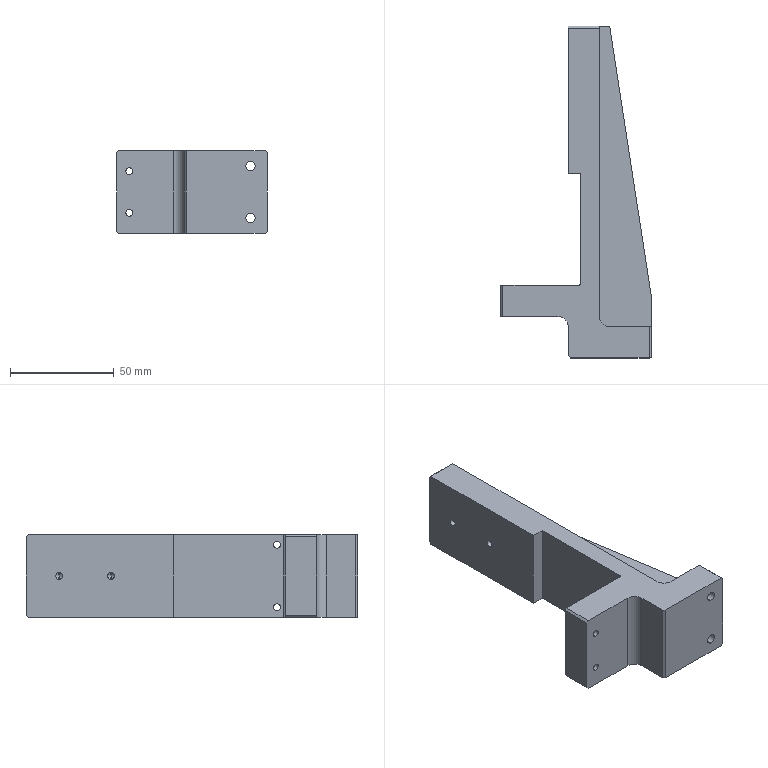Part | SolidWorks | features HoleWzd 3, ICE 3, Fillet 2, Chamfer 1, Extrusion 1 | 1 solid | 50 faces | box 72.5 x 160 x 40 mm | volume 135380 mm3 | plane 26 | cylinder 20 | cone 4 | commonest cylinder face diameters 3.3 x12 4.5 x4 10 x3 2 x1
STEP:
#1=CARTESIAN_POINT('',(47.5,4.,-16.65));
#2=VERTEX_POINT('',#1);
#3=CARTESIAN_POINT('',(47.5,4.,-13.35));
#4=VERTEX_POINT('',#3);
#5=CARTESIAN_POINT('',(47.5,4.,-15.));
#6=DIRECTION('',(-1.,0.,0.));
#7=DIRECTION('',(0.,-1.,0.));
#8=AXIS2_PLACEMENT_3D('',#5,#6,#7);
#9=CIRCLE('',#8,1.65);
#10=EDGE_CURVE('',#2,#4,#9,.T.);
#11=ORIENTED_EDGE('',*,*,#10,.F.);
#12=CARTESIAN_POINT('',(38.5,4.,-16.65));
#13=VERTEX_POINT('',#12);
#14=CARTESIAN_POINT('',(38.5,4.,-16.65));
#15=DIRECTION('',(-1.,0.,0.));
#16=VECTOR('',#15,1000.);
#17=LINE('',#14,#16);
#18=EDGE_CURVE('',#2,#13,#17,.T.);
#19=ORIENTED_EDGE('',*,*,#18,.T.);
#20=CARTESIAN_POINT('',(38.5,4.,-13.35));
#21=VERTEX_POINT('',#20);
#22=CARTESIAN_POINT('',(38.5,4.,-15.));
#23=DIRECTION('',(-1.,0.,0.));
#24=DIRECTION('',(0.,0.,1.));
#25=AXIS2_PLACEMENT_3D('',#22,#23,#24);
#26=CIRCLE('',#25,1.65);
#27=EDGE_CURVE('',#13,#21,#26,.T.);
#28=ORIENTED_EDGE('',*,*,#27,.T.);
#29=CARTESIAN_POINT('',(38.5,4.,-13.35));
#30=DIRECTION('',(-1.,0.,0.));
#31=VECTOR('',#30,1000.);
#32=LINE('',#29,#31);
#33=EDGE_CURVE('',#4,#21,#32,.T.);
#34=ORIENTED_EDGE('',*,*,#33,.F.);
#35=EDGE_LOOP('',(#11,#19,#28,#34));
#36=FACE_OUTER_BOUND('',#35,.T.);
#37=CARTESIAN_POINT('',(38.5,4.,-15.));
#38=DIRECTION('',(-1.,0.,0.));
#39=DIRECTION('',(0.,0.,1.));
#40=AXIS2_PLACEMENT_3D('',#37,#38,#39);
#41=CYLINDRICAL_SURFACE('',#40,1.65);
#42=ADVANCED_FACE('',(#36),#41,.F.);
#43=CARTESIAN_POINT('',(47.5,4.,13.35));
#44=VERTEX_POINT('',#43);
#45=CARTESIAN_POINT('',(47.5,4.,16.65));
#46=VERTEX_POINT('',#45);
#47=CARTESIAN_POINT('',(47.5,4.,15.));
#48=DIRECTION('',(-1.,0.,0.));
#49=DIRECTION('',(0.,-1.,0.));
#50=AXIS2_PLACEMENT_3D('',#47,#48,#49);
#51=CIRCLE('',#50,1.65);
#52=EDGE_CURVE('',#44,#46,#51,.T.);
#53=ORIENTED_EDGE('',*,*,#52,.F.);
#54=CARTESIAN_POINT('',(38.5,4.,13.35));
#55=VERTEX_POINT('',#54);
#56=CARTESIAN_POINT('',(38.5,4.,13.35));
#57=DIRECTION('',(-1.,0.,0.));
#58=VECTOR('',#57,1000.);
#59=LINE('',#56,#58);
#60=EDGE_CURVE('',#44,#55,#59,.T.);
#61=ORIENTED_EDGE('',*,*,#60,.T.);
#62=CARTESIAN_POINT('',(38.5,4.,16.65));
#63=VERTEX_POINT('',#62);
#64=CARTESIAN_POINT('',(38.5,4.,15.));
#65=DIRECTION('',(-1.,0.,0.));
#66=DIRECTION('',(0.,0.,1.));
#67=AXIS2_PLACEMENT_3D('',#64,#65,#66);
#68=CIRCLE('',#67,1.65);
#69=EDGE_CURVE('',#55,#63,#68,.T.);
#70=ORIENTED_EDGE('',*,*,#69,.T.);
#71=CARTESIAN_POINT('',(38.5,4.,16.65));
#72=DIRECTION('',(-1.,0.,0.));
#73=VECTOR('',#72,1000.);
#74=LINE('',#71,#73);
#75=EDGE_CURVE('',#46,#63,#74,.T.);
#76=ORIENTED_EDGE('',*,*,#75,.F.);
#77=EDGE_LOOP('',(#53,#61,#70,#76));
#78=FACE_OUTER_BOUND('',#77,.T.);
#79=CARTESIAN_POINT('',(38.5,4.,15.));
#80=DIRECTION('',(-1.,0.,0.));
#81=DIRECTION('',(0.,0.,1.));
#82=AXIS2_PLACEMENT_3D('',#79,#80,#81);
#83=CYLINDRICAL_SURFACE('',#82,1.65);
#84=ADVANCED_FACE('',(#78),#83,.F.);
#85=CARTESIAN_POINT('',(44.,109.,-1.65));
#86=VERTEX_POINT('',#85);
#87=CARTESIAN_POINT('',(44.,109.,1.65));
#88=VERTEX_POINT('',#87);
#89=CARTESIAN_POINT('',(44.,109.,0.));
#90=DIRECTION('',(-1.,0.,0.));
#91=DIRECTION('',(0.,0.,1.));
#92=AXIS2_PLACEMENT_3D('',#89,#90,#91);
#93=CIRCLE('',#92,1.65);
#94=EDGE_CURVE('',#86,#88,#93,.T.);
#95=ORIENTED_EDGE('',*,*,#94,.F.);
#96=CARTESIAN_POINT('',(32.5,109.,-1.65));
#97=VERTEX_POINT('',#96);
#98=CARTESIAN_POINT('',(32.5,109.,-1.65));
#99=DIRECTION('',(-1.,0.,0.));
#100=VECTOR('',#99,1000.);
#101=LINE('',#98,#100);
#102=EDGE_CURVE('',#86,#97,#101,.T.);
#103=ORIENTED_EDGE('',*,*,#102,.T.);
#104=CARTESIAN_POINT('',(32.5,109.,1.65));
#105=VERTEX_POINT('',#104);
#106=CARTESIAN_POINT('',(32.5,109.,0.));
#107=DIRECTION('',(-1.,0.,0.));
#108=DIRECTION('',(0.,0.,1.));
#109=AXIS2_PLACEMENT_3D('',#106,#107,#108);
#110=CIRCLE('',#109,1.65);
#111=EDGE_CURVE('',#97,#105,#110,.T.);
#112=ORIENTED_EDGE('',*,*,#111,.T.);
#113=CARTESIAN_POINT('',(32.5,109.,1.65));
#114=DIRECTION('',(-1.,0.,0.));
#115=VECTOR('',#114,1000.);
#116=LINE('',#113,#115);
#117=EDGE_CURVE('',#88,#105,#116,.T.);
#118=ORIENTED_EDGE('',*,*,#117,.F.);
#119=EDGE_LOOP('',(#95,#103,#112,#118));
#120=FACE_OUTER_BOUND('',#119,.T.);
#121=CARTESIAN_POINT('',(32.5,109.,0.));
#122=DIRECTION('',(-1.,0.,0.));
#123=DIRECTION('',(0.,0.,1.));
#124=AXIS2_PLACEMENT_3D('',#121,#122,#123);
#125=CYLINDRICAL_SURFACE('',#124,1.65);
#126=ADVANCED_FACE('',(#120),#125,.F.);
#127=CARTESIAN_POINT('',(44.991,109.,0.));
#128=VERTEX_POINT('',#127);
#129=CARTESIAN_POINT('',(44.,109.,1.65));
#130=DIRECTION('',(-0.515,0.,0.8572));
#131=VECTOR('',#130,1000.);
#132=LINE('',#129,#131);
#133=EDGE_CURVE('',#128,#88,#132,.T.);
#134=ORIENTED_EDGE('',*,*,#133,.F.);
#135=CARTESIAN_POINT('',(44.,109.,-1.65));
#136=DIRECTION('',(-0.515,0.,-0.8572));
#137=VECTOR('',#136,1000.);
#138=LINE('',#135,#137);
#139=EDGE_CURVE('',#128,#86,#138,.T.);
#140=ORIENTED_EDGE('',*,*,#139,.T.);
#141=ORIENTED_EDGE('',*,*,#94,.T.);
#142=EDGE_LOOP('',(#134,#140,#141));
#143=FACE_OUTER_BOUND('',#142,.T.);
#144=CARTESIAN_POINT('',(44.,109.,0.));
#145=DIRECTION('',(-1.,0.,0.));
#146=DIRECTION('',(0.,0.,1.));
#147=AXIS2_PLACEMENT_3D('',#144,#145,#146);
#148=CONICAL_SURFACE('',#147,1.65,1.03);
#149=ADVANCED_FACE('',(#143),#148,.F.);
#150=CARTESIAN_POINT('',(44.,84.,-1.65));
#151=VERTEX_POINT('',#150);
#152=CARTESIAN_POINT('',(44.,84.,1.65));
#153=VERTEX_POINT('',#152);
#154=CARTESIAN_POINT('',(44.,84.,0.));
#155=DIRECTION('',(-1.,0.,0.));
#156=DIRECTION('',(0.,0.,1.));
#157=AXIS2_PLACEMENT_3D('',#154,#155,#156);
#158=CIRCLE('',#157,1.65);
#159=EDGE_CURVE('',#151,#153,#158,.T.);
#160=ORIENTED_EDGE('',*,*,#159,.F.);
#161=CARTESIAN_POINT('',(32.5,84.,-1.65));
#162=VERTEX_POINT('',#161);
#163=CARTESIAN_POINT('',(32.5,84.,-1.65));
#164=DIRECTION('',(-1.,0.,0.));
#165=VECTOR('',#164,1000.);
#166=LINE('',#163,#165);
#167=EDGE_CURVE('',#151,#162,#166,.T.);
#168=ORIENTED_EDGE('',*,*,#167,.T.);
#169=CARTESIAN_POINT('',(32.5,84.,1.65));
#170=VERTEX_POINT('',#169);
#171=CARTESIAN_POINT('',(32.5,84.,0.));
#172=DIRECTION('',(-1.,0.,0.));
#173=DIRECTION('',(0.,0.,1.));
#174=AXIS2_PLACEMENT_3D('',#171,#172,#173);
#175=CIRCLE('',#174,1.65);
#176=EDGE_CURVE('',#162,#170,#175,.T.);
#177=ORIENTED_EDGE('',*,*,#176,.T.);
#178=CARTESIAN_POINT('',(32.5,84.,1.65));
#179=DIRECTION('',(-1.,0.,0.));
#180=VECTOR('',#179,1000.);
#181=LINE('',#178,#180);
#182=EDGE_CURVE('',#153,#170,#181,.T.);
#183=ORIENTED_EDGE('',*,*,#182,.F.);
#184=EDGE_LOOP('',(#160,#168,#177,#183));
#185=FACE_OUTER_BOUND('',#184,.T.);
#186=CARTESIAN_POINT('',(32.5,84.,0.));
#187=DIRECTION('',(-1.,0.,0.));
#188=DIRECTION('',(0.,0.,1.));
#189=AXIS2_PLACEMENT_3D('',#186,#187,#188);
#190=CYLINDRICAL_SURFACE('',#189,1.65);
#191=ADVANCED_FACE('',(#185),#190,.F.);
#192=CARTESIAN_POINT('',(44.991,84.,0.));
#193=VERTEX_POINT('',#192);
#194=CARTESIAN_POINT('',(44.,84.,1.65));
#195=DIRECTION('',(-0.515,0.,0.8572));
#196=VECTOR('',#195,1000.);
#197=LINE('',#194,#196);
#198=EDGE_CURVE('',#193,#153,#197,.T.);
#199=ORIENTED_EDGE('',*,*,#198,.F.);
#200=CARTESIAN_POINT('',(44.,84.,-1.65));
#201=DIRECTION('',(-0.515,0.,-0.8572));
#202=VECTOR('',#201,1000.);
#203=LINE('',#200,#202);
#204=EDGE_CURVE('',#193,#151,#203,.T.);
#205=ORIENTED_EDGE('',*,*,#204,.T.);
#206=ORIENTED_EDGE('',*,*,#159,.T.);
#207=EDGE_LOOP('',(#199,#205,#206));
#208=FACE_OUTER_BOUND('',#207,.T.);
#209=CARTESIAN_POINT('',(44.,84.,0.));
#210=DIRECTION('',(-1.,0.,0.));
#211=DIRECTION('',(0.,0.,1.));
#212=AXIS2_PLACEMENT_3D('',#209,#210,#211);
#213=CONICAL_SURFACE('',#212,1.65,1.03);
#214=ADVANCED_FACE('',(#208),#213,.F.);
#215=CARTESIAN_POINT('',(6.,-15.,-11.65));
#216=VERTEX_POINT('',#215);
#217=CARTESIAN_POINT('',(6.,-15.,-8.35));
#218=VERTEX_POINT('',#217);
#219=CARTESIAN_POINT('',(6.,-15.,-10.));
#220=DIRECTION('',(0.,1.,0.));
#221=DIRECTION('',(0.,0.,1.));
#222=AXIS2_PLACEMENT_3D('',#219,#220,#221);
#223=CIRCLE('',#222,1.65);
#224=EDGE_CURVE('',#216,#218,#223,.T.);
#225=ORIENTED_EDGE('',*,*,#224,.F.);
#226=CARTESIAN_POINT('',(6.,0.,-11.65));
#227=VERTEX_POINT('',#226);
#228=CARTESIAN_POINT('',(6.,0.,-11.65));
#229=DIRECTION('',(0.,1.,0.));
#230=VECTOR('',#229,1000.);
#231=LINE('',#228,#230);
#232=EDGE_CURVE('',#216,#227,#231,.T.);
#233=ORIENTED_EDGE('',*,*,#232,.T.);
#234=CARTESIAN_POINT('',(6.,0.,-8.35));
#235=VERTEX_POINT('',#234);
#236=CARTESIAN_POINT('',(6.,0.,-10.));
#237=DIRECTION('',(0.,1.,0.));
#238=DIRECTION('',(0.,0.,1.));
#239=AXIS2_PLACEMENT_3D('',#236,#237,#238);
#240=CIRCLE('',#239,1.65);
#241=EDGE_CURVE('',#227,#235,#240,.T.);
#242=ORIENTED_EDGE('',*,*,#241,.T.);
#243=CARTESIAN_POINT('',(6.,0.,-8.35));
#244=DIRECTION('',(0.,1.,0.));
#245=VECTOR('',#244,1000.);
#246=LINE('',#243,#245);
#247=EDGE_CURVE('',#218,#235,#246,.T.);
#248=ORIENTED_EDGE('',*,*,#247,.F.);
#249=EDGE_LOOP('',(#225,#233,#242,#248));
#250=FACE_OUTER_BOUND('',#249,.T.);
#251=CARTESIAN_POINT('',(6.,0.,-10.));
#252=DIRECTION('',(0.,1.,0.));
#253=DIRECTION('',(0.,0.,1.));
#254=AXIS2_PLACEMENT_3D('',#251,#252,#253);
#255=CYLINDRICAL_SURFACE('',#254,1.65);
#256=ADVANCED_FACE('',(#250),#255,.F.);
#257=CARTESIAN_POINT('',(6.,-15.,8.35));
#258=VERTEX_POINT('',#257);
#259=CARTESIAN_POINT('',(6.,-15.,11.65));
#260=VERTEX_POINT('',#259);
#261=CARTESIAN_POINT('',(6.,-15.,10.));
#262=DIRECTION('',(0.,1.,0.));
#263=DIRECTION('',(0.,0.,1.));
#264=AXIS2_PLACEMENT_3D('',#261,#262,#263);
#265=CIRCLE('',#264,1.65);
#266=EDGE_CURVE('',#258,#260,#265,.T.);
#267=ORIENTED_EDGE('',*,*,#266,.F.);
#268=CARTESIAN_POINT('',(6.,0.,8.35));
#269=VERTEX_POINT('',#268);
#270=CARTESIAN_POINT('',(6.,0.,8.35));
#271=DIRECTION('',(0.,1.,0.));
#272=VECTOR('',#271,1000.);
#273=LINE('',#270,#272);
#274=EDGE_CURVE('',#258,#269,#273,.T.);
#275=ORIENTED_EDGE('',*,*,#274,.T.);
#276=CARTESIAN_POINT('',(6.,0.,11.65));
#277=VERTEX_POINT('',#276);
#278=CARTESIAN_POINT('',(6.,0.,10.));
#279=DIRECTION('',(0.,1.,0.));
#280=DIRECTION('',(0.,0.,1.));
#281=AXIS2_PLACEMENT_3D('',#278,#279,#280);
#282=CIRCLE('',#281,1.65);
#283=EDGE_CURVE('',#269,#277,#282,.T.);
#284=ORIENTED_EDGE('',*,*,#283,.T.);
#285=CARTESIAN_POINT('',(6.,0.,11.65));
#286=DIRECTION('',(0.,1.,0.));
#287=VECTOR('',#286,1000.);
#288=LINE('',#285,#287);
#289=EDGE_CURVE('',#260,#277,#288,.T.);
#290=ORIENTED_EDGE('',*,*,#289,.F.);
#291=EDGE_LOOP('',(#267,#275,#284,#290));
#292=FACE_OUTER_BOUND('',#291,.T.);
#293=CARTESIAN_POINT('',(6.,0.,10.));
#294=DIRECTION('',(0.,1.,0.));
#295=DIRECTION('',(0.,0.,1.));
#296=AXIS2_PLACEMENT_3D('',#293,#294,#295);
#297=CYLINDRICAL_SURFACE('',#296,1.65);
#298=ADVANCED_FACE('',(#292),#297,.F.);
#299=CARTESIAN_POINT('',(64.5,-35.,-14.75));
#300=VERTEX_POINT('',#299);
#301=CARTESIAN_POINT('',(64.5,-35.,-10.25));
#302=VERTEX_POINT('',#301);
#303=CARTESIAN_POINT('',(64.5,-35.,-12.5));
#304=DIRECTION('',(0.,1.,0.));
#305=DIRECTION('',(0.,0.,1.));
#306=AXIS2_PLACEMENT_3D('',#303,#304,#305);
#307=CIRCLE('',#306,2.25);
#308=EDGE_CURVE('',#300,#302,#307,.T.);
#309=ORIENTED_EDGE('',*,*,#308,.F.);
#310=CARTESIAN_POINT('',(64.5,-20.,-14.75));
#311=VERTEX_POINT('',#310);
#312=CARTESIAN_POINT('',(64.5,-35.,-14.75));
#313=DIRECTION('',(0.,1.,0.));
#314=VECTOR('',#313,1000.);
#315=LINE('',#312,#314);
#316=EDGE_CURVE('',#300,#311,#315,.T.);
#317=ORIENTED_EDGE('',*,*,#316,.T.);
#318=CARTESIAN_POINT('',(64.5,-20.,-10.25));
#319=VERTEX_POINT('',#318);
#320=CARTESIAN_POINT('',(64.5,-20.,-12.5));
#321=DIRECTION('',(0.,1.,0.));
#322=DIRECTION('',(0.,0.,1.));
#323=AXIS2_PLACEMENT_3D('',#320,#321,#322);
#324=CIRCLE('',#323,2.25);
#325=EDGE_CURVE('',#311,#319,#324,.T.);
#326=ORIENTED_EDGE('',*,*,#325,.T.);
#327=CARTESIAN_POINT('',(64.5,-35.,-10.25));
#328=DIRECTION('',(0.,1.,0.));
#329=VECTOR('',#328,1000.);
#330=LINE('',#327,#329);
#331=EDGE_CURVE('',#302,#319,#330,.T.);
#332=ORIENTED_EDGE('',*,*,#331,.F.);
#333=EDGE_LOOP('',(#309,#317,#326,#332));
#334=FACE_OUTER_BOUND('',#333,.T.);
#335=CARTESIAN_POINT('',(64.5,-35.,-12.5));
#336=DIRECTION('',(0.,1.,0.));
#337=DIRECTION('',(0.,0.,1.));
#338=AXIS2_PLACEMENT_3D('',#335,#336,#337);
#339=CYLINDRICAL_SURFACE('',#338,2.25);
#340=ADVANCED_FACE('',(#334),#339,.F.);
#341=CARTESIAN_POINT('',(64.5,-35.,10.25));
#342=VERTEX_POINT('',#341);
#343=CARTESIAN_POINT('',(64.5,-35.,14.75));
#344=VERTEX_POINT('',#343);
#345=CARTESIAN_POINT('',(64.5,-35.,12.5));
#346=DIRECTION('',(0.,1.,0.));
#347=DIRECTION('',(0.,0.,1.));
#348=AXIS2_PLACEMENT_3D('',#345,#346,#347);
#349=CIRCLE('',#348,2.25);
#350=EDGE_CURVE('',#342,#344,#349,.T.);
#351=ORIENTED_EDGE('',*,*,#350,.F.);
#352=CARTESIAN_POINT('',(64.5,-20.,10.25));
#353=VERTEX_POINT('',#352);
#354=CARTESIAN_POINT('',(64.5,-35.,10.25));
#355=DIRECTION('',(0.,1.,0.));
#356=VECTOR('',#355,1000.);
#357=LINE('',#354,#356);
#358=EDGE_CURVE('',#342,#353,#357,.T.);
#359=ORIENTED_EDGE('',*,*,#358,.T.);
#360=CARTESIAN_POINT('',(64.5,-20.,14.75));
#361=VERTEX_POINT('',#360);
#362=CARTESIAN_POINT('',(64.5,-20.,12.5));
#363=DIRECTION('',(0.,1.,0.));
#364=DIRECTION('',(0.,0.,1.));
#365=AXIS2_PLACEMENT_3D('',#362,#363,#364);
#366=CIRCLE('',#365,2.25);
#367=EDGE_CURVE('',#353,#361,#366,.T.);
#368=ORIENTED_EDGE('',*,*,#367,.T.);
#369=CARTESIAN_POINT('',(64.5,-35.,14.75));
#370=DIRECTION('',(0.,1.,0.));
#371=VECTOR('',#370,1000.);
#372=LINE('',#369,#371);
#373=EDGE_CURVE('',#344,#361,#372,.T.);
#374=ORIENTED_EDGE('',*,*,#373,.F.);
#375=EDGE_LOOP('',(#351,#359,#368,#374));
#376=FACE_OUTER_BOUND('',#375,.T.);
#377=CARTESIAN_POINT('',(64.5,-35.,12.5));
#378=DIRECTION('',(0.,1.,0.));
#379=DIRECTION('',(0.,0.,1.));
#380=AXIS2_PLACEMENT_3D('',#377,#378,#379);
#381=CYLINDRICAL_SURFACE('',#380,2.25);
#382=ADVANCED_FACE('',(#376),#381,.F.);
#383=CARTESIAN_POINT('',(64.5,-20.,12.5));
#384=DIRECTION('',(0.,1.,0.));
#385=DIRECTION('',(0.,0.,1.));
#386=AXIS2_PLACEMENT_3D('',#383,#384,#385);
#387=CIRCLE('',#386,2.25);
#388=EDGE_CURVE('',#361,#353,#387,.T.);
#389=ORIENTED_EDGE('',*,*,#388,.F.);
#390=ORIENTED_EDGE('',*,*,#367,.F.);
#391=EDGE_LOOP('',(#389,#390));
#392=FACE_BOUND('',#391,.T.);
#393=CARTESIAN_POINT('',(52.5,-20.,4.));
#394=VERTEX_POINT('',#393);
#395=CARTESIAN_POINT('',(72.5,-20.,4.));
#396=VERTEX_POINT('',#395);
#397=CARTESIAN_POINT('',(72.5,-20.,4.));
#398=DIRECTION('',(1.,0.,0.));
#399=VECTOR('',#398,1000.);
#400=LINE('',#397,#399);
#401=EDGE_CURVE('',#394,#396,#400,.T.);
#402=ORIENTED_EDGE('',*,*,#401,.F.);
#403=CARTESIAN_POINT('',(52.5,-20.,20.));
#404=VERTEX_POINT('',#403);
#405=CARTESIAN_POINT('',(52.5,-20.,20.));
#406=DIRECTION('',(0.,0.,1.));
#407=VECTOR('',#406,1000.);
#408=LINE('',#405,#407);
#409=EDGE_CURVE('',#394,#404,#408,.T.);
#410=ORIENTED_EDGE('',*,*,#409,.T.);
#411=CARTESIAN_POINT('',(71.5,-20.,20.));
#412=VERTEX_POINT('',#411);
#413=CARTESIAN_POINT('',(47.5,-20.,20.));
#414=DIRECTION('',(-1.,0.,0.));
#415=VECTOR('',#414,1000.);
#416=LINE('',#413,#415);
#417=EDGE_CURVE('',#412,#404,#416,.T.);
#418=ORIENTED_EDGE('',*,*,#417,.F.);
#419=CARTESIAN_POINT('',(72.5,-20.,19.));
#420=VERTEX_POINT('',#419);
#421=CARTESIAN_POINT('',(71.5,-20.,20.));
#422=DIRECTION('',(0.7071,0.,-0.7071));
#423=VECTOR('',#422,1000.);
#424=LINE('',#421,#423);
#425=EDGE_CURVE('',#412,#420,#424,.T.);
#426=ORIENTED_EDGE('',*,*,#425,.T.);
#427=CARTESIAN_POINT('',(72.5,-20.,20.));
#428=DIRECTION('',(0.,0.,-1.));
#429=VECTOR('',#428,1000.);
#430=LINE('',#427,#429);
#431=EDGE_CURVE('',#420,#396,#430,.T.);
#432=ORIENTED_EDGE('',*,*,#431,.T.);
#433=EDGE_LOOP('',(#402,#410,#418,#426,#432));
#434=FACE_OUTER_BOUND('',#433,.T.);
#435=CARTESIAN_POINT('',(47.5,-20.,20.));
#436=DIRECTION('',(0.,-1.,0.));
#437=DIRECTION('',(0.,0.,-1.));
#438=AXIS2_PLACEMENT_3D('',#435,#436,#437);
#439=PLANE('',#438);
#440=ADVANCED_FACE('',(#392,#434),#439,.F.);
#441=CARTESIAN_POINT('',(47.5,4.,15.));
#442=DIRECTION('',(-1.,0.,0.));
#443=DIRECTION('',(0.,-1.,0.));
#444=AXIS2_PLACEMENT_3D('',#441,#442,#443);
#445=CIRCLE('',#444,1.65);
#446=EDGE_CURVE('',#46,#44,#445,.T.);
#447=ORIENTED_EDGE('',*,*,#446,.T.);
#448=ORIENTED_EDGE('',*,*,#52,.T.);
#449=EDGE_LOOP('',(#447,#448));
#450=FACE_BOUND('',#449,.T.);
#451=CARTESIAN_POINT('',(47.5,-15.,20.));
#452=VERTEX_POINT('',#451);
#453=CARTESIAN_POINT('',(47.5,124.,20.));
#454=VERTEX_POINT('',#453);
#455=CARTESIAN_POINT('',(47.5,125.,20.));
#456=DIRECTION('',(0.,1.,0.));
#457=VECTOR('',#456,1000.);
#458=LINE('',#455,#457);
#459=EDGE_CURVE('',#452,#454,#458,.T.);
#460=ORIENTED_EDGE('',*,*,#459,.F.);
#461=CARTESIAN_POINT('',(47.5,-15.,4.));
#462=VERTEX_POINT('',#461);
#463=CARTESIAN_POINT('',(47.5,-15.,4.));
#464=DIRECTION('',(0.,0.,-1.));
#465=VECTOR('',#464,1000.);
#466=LINE('',#463,#465);
#467=EDGE_CURVE('',#452,#462,#466,.T.);
#468=ORIENTED_EDGE('',*,*,#467,.T.);
#469=CARTESIAN_POINT('',(47.5,125.,4.));
#470=VERTEX_POINT('',#469);
#471=CARTESIAN_POINT('',(47.5,-20.,4.));
#472=DIRECTION('',(0.,-1.,0.));
#473=VECTOR('',#472,1000.);
#474=LINE('',#471,#473);
#475=EDGE_CURVE('',#470,#462,#474,.T.);
#476=ORIENTED_EDGE('',*,*,#475,.F.);
#477=CARTESIAN_POINT('',(47.5,125.,19.));
#478=VERTEX_POINT('',#477);
#479=CARTESIAN_POINT('',(47.5,125.,20.));
#480=DIRECTION('',(0.,0.,-1.));
#481=VECTOR('',#480,1000.);
#482=LINE('',#479,#481);
#483=EDGE_CURVE('',#478,#470,#482,.T.);
#484=ORIENTED_EDGE('',*,*,#483,.F.);
#485=CARTESIAN_POINT('',(47.5,124.,20.));
#486=DIRECTION('',(0.,-0.7071,0.7071));
#487=VECTOR('',#486,1000.);
#488=LINE('',#485,#487);
#489=EDGE_CURVE('',#478,#454,#488,.T.);
#490=ORIENTED_EDGE('',*,*,#489,.T.);
#491=EDGE_LOOP('',(#460,#468,#476,#484,#490));
#492=FACE_OUTER_BOUND('',#491,.T.);
#493=CARTESIAN_POINT('',(47.5,125.,20.));
#494=DIRECTION('',(-1.,0.,0.));
#495=DIRECTION('',(0.,-1.,0.));
#496=AXIS2_PLACEMENT_3D('',#493,#494,#495);
#497=PLANE('',#496);
#498=ADVANCED_FACE('',(#450,#492),#497,.F.);
#499=CARTESIAN_POINT('',(0.,0.,19.));
#500=VERTEX_POINT('',#499);
#501=CARTESIAN_POINT('',(0.,0.,-19.));
#502=VERTEX_POINT('',#501);
#503=CARTESIAN_POINT('',(0.,0.,20.));
#504=DIRECTION('',(0.,0.,-1.));
#505=VECTOR('',#504,1000.);
#506=LINE('',#503,#505);
#507=EDGE_CURVE('',#500,#502,#506,.T.);
#508=ORIENTED_EDGE('',*,*,#507,.T.);
#509=CARTESIAN_POINT('',(0.,-15.,-19.));
#510=VERTEX_POINT('',#509);
#511=CARTESIAN_POINT('',(0.,-15.,-19.));
#512=DIRECTION('',(0.,-1.,0.));
#513=VECTOR('',#512,1000.);
#514=LINE('',#511,#513);
#515=EDGE_CURVE('',#502,#510,#514,.T.);
#516=ORIENTED_EDGE('',*,*,#515,.T.);
#517=CARTESIAN_POINT('',(0.,-15.,19.));
#518=VERTEX_POINT('',#517);
#519=CARTESIAN_POINT('',(0.,-15.,20.));
#520=DIRECTION('',(0.,0.,-1.));
#521=VECTOR('',#520,1000.);
#522=LINE('',#519,#521);
#523=EDGE_CURVE('',#518,#510,#522,.T.);
#524=ORIENTED_EDGE('',*,*,#523,.F.);
#525=CARTESIAN_POINT('',(0.,-15.,19.));
#526=DIRECTION('',(0.,1.,0.));
#527=VECTOR('',#526,1000.);
#528=LINE('',#525,#527);
#529=EDGE_CURVE('',#518,#500,#528,.T.);
#530=ORIENTED_EDGE('',*,*,#529,.T.);
#531=EDGE_LOOP('',(#508,#516,#524,#530));
#532=FACE_OUTER_BOUND('',#531,.T.);
#533=CARTESIAN_POINT('',(0.,-15.,20.));
#534=DIRECTION('',(1.,0.,0.));
#535=DIRECTION('',(0.,0.,-1.));
#536=AXIS2_PLACEMENT_3D('',#533,#534,#535);
#537=PLANE('',#536);
#538=ADVANCED_FACE('',(#532),#537,.F.);
#539=CARTESIAN_POINT('',(6.,-15.,-10.));
#540=DIRECTION('',(0.,1.,0.));
#541=DIRECTION('',(0.,0.,1.));
#542=AXIS2_PLACEMENT_3D('',#539,#540,#541);
#543=CIRCLE('',#542,1.65);
#544=EDGE_CURVE('',#218,#216,#543,.T.);
#545=ORIENTED_EDGE('',*,*,#544,.T.);
#546=ORIENTED_EDGE('',*,*,#224,.T.);
#547=EDGE_LOOP('',(#545,#546));
#548=FACE_BOUND('',#547,.T.);
#549=CARTESIAN_POINT('',(6.,-15.,10.));
#550=DIRECTION('',(0.,1.,0.));
#551=DIRECTION('',(0.,0.,1.));
#552=AXIS2_PLACEMENT_3D('',#549,#550,#551);
#553=CIRCLE('',#552,1.65);
#554=EDGE_CURVE('',#260,#258,#553,.T.);
#555=ORIENTED_EDGE('',*,*,#554,.T.);
#556=ORIENTED_EDGE('',*,*,#266,.T.);
#557=EDGE_LOOP('',(#555,#556));
#558=FACE_BOUND('',#557,.T.);
#559=CARTESIAN_POINT('',(1.,-15.,-20.));
#560=VERTEX_POINT('',#559);
#561=CARTESIAN_POINT('',(27.5,-15.,-20.));
#562=VERTEX_POINT('',#561);
#563=CARTESIAN_POINT('',(0.,-15.,-20.));
#564=DIRECTION('',(1.,0.,0.));
#565=VECTOR('',#564,1000.);
#566=LINE('',#563,#565);
#567=EDGE_CURVE('',#560,#562,#566,.T.);
#568=ORIENTED_EDGE('',*,*,#567,.T.);
#569=CARTESIAN_POINT('',(27.5,-15.,20.));
#570=VERTEX_POINT('',#569);
#571=CARTESIAN_POINT('',(27.5,-15.,20.));
#572=DIRECTION('',(0.,0.,1.));
#573=VECTOR('',#572,1000.);
#574=LINE('',#571,#573);
#575=EDGE_CURVE('',#562,#570,#574,.T.);
#576=ORIENTED_EDGE('',*,*,#575,.T.);
#577=CARTESIAN_POINT('',(1.,-15.,20.));
#578=VERTEX_POINT('',#577);
#579=CARTESIAN_POINT('',(0.,-15.,20.));
#580=DIRECTION('',(1.,0.,0.));
#581=VECTOR('',#580,1000.);
#582=LINE('',#579,#581);
#583=EDGE_CURVE('',#578,#570,#582,.T.);
#584=ORIENTED_EDGE('',*,*,#583,.F.);
#585=CARTESIAN_POINT('',(1.,-15.,20.));
#586=DIRECTION('',(-0.7071,0.,-0.7071));
#587=VECTOR('',#586,1000.);
#588=LINE('',#585,#587);
#589=EDGE_CURVE('',#578,#518,#588,.T.);
#590=ORIENTED_EDGE('',*,*,#589,.T.);
#591=ORIENTED_EDGE('',*,*,#523,.T.);
#592=CARTESIAN_POINT('',(0.,-15.,-19.));
#593=DIRECTION('',(0.7071,0.,-0.7071));
#594=VECTOR('',#593,1000.);
#595=LINE('',#592,#594);
#596=EDGE_CURVE('',#510,#560,#595,.T.);
#597=ORIENTED_EDGE('',*,*,#596,.T.);
#598=EDGE_LOOP('',(#568,#576,#584,#590,#591,#597));
#599=FACE_OUTER_BOUND('',#598,.T.);
#600=CARTESIAN_POINT('',(0.,-15.,20.));
#601=DIRECTION('',(0.,1.,0.));
#602=DIRECTION('',(0.,0.,1.));
#603=AXIS2_PLACEMENT_3D('',#600,#601,#602);
#604=PLANE('',#603);
#605=ADVANCED_FACE('',(#548,#558,#599),#604,.F.);
#606=CARTESIAN_POINT('',(32.5,-20.,20.));
#607=VERTEX_POINT('',#606);
#608=CARTESIAN_POINT('',(32.5,-34.,20.));
#609=VERTEX_POINT('',#608);
#610=CARTESIAN_POINT('',(32.5,-15.,20.));
#611=DIRECTION('',(0.,-1.,0.));
#612=VECTOR('',#611,1000.);
#613=LINE('',#610,#612);
#614=EDGE_CURVE('',#607,#609,#613,.T.);
#615=ORIENTED_EDGE('',*,*,#614,.F.);
#616=CARTESIAN_POINT('',(32.5,-20.,-20.));
#617=VERTEX_POINT('',#616);
#618=CARTESIAN_POINT('',(32.5,-20.,-20.));
#619=DIRECTION('',(0.,0.,-1.));
#620=VECTOR('',#619,1000.);
#621=LINE('',#618,#620);
#622=EDGE_CURVE('',#607,#617,#621,.T.);
#623=ORIENTED_EDGE('',*,*,#622,.T.);
#624=CARTESIAN_POINT('',(32.5,-34.,-20.));
#625=VERTEX_POINT('',#624);
#626=CARTESIAN_POINT('',(32.5,-15.,-20.));
#627=DIRECTION('',(0.,-1.,0.));
#628=VECTOR('',#627,1000.);
#629=LINE('',#626,#628);
#630=EDGE_CURVE('',#617,#625,#629,.T.);
#631=ORIENTED_EDGE('',*,*,#630,.T.);
#632=CARTESIAN_POINT('',(32.5,-34.,20.));
#633=DIRECTION('',(0.,0.,1.));
#634=VECTOR('',#633,1000.);
#635=LINE('',#632,#634);
#636=EDGE_CURVE('',#625,#609,#635,.T.);
#637=ORIENTED_EDGE('',*,*,#636,.T.);
#638=EDGE_LOOP('',(#615,#623,#631,#637));
#639=FACE_OUTER_BOUND('',#638,.T.);
#640=CARTESIAN_POINT('',(32.5,-15.,20.));
#641=DIRECTION('',(1.,0.,0.));
#642=DIRECTION('',(0.,0.,-1.));
#643=AXIS2_PLACEMENT_3D('',#640,#641,#642);
#644=PLANE('',#643);
#645=ADVANCED_FACE('',(#639),#644,.F.);
#646=CARTESIAN_POINT('',(64.5,-35.,-12.5));
#647=DIRECTION('',(0.,1.,0.));
#648=DIRECTION('',(0.,0.,1.));
#649=AXIS2_PLACEMENT_3D('',#646,#647,#648);
#650=CIRCLE('',#649,2.25);
#651=EDGE_CURVE('',#302,#300,#650,.T.);
#652=ORIENTED_EDGE('',*,*,#651,.T.);
#653=ORIENTED_EDGE('',*,*,#308,.T.);
#654=EDGE_LOOP('',(#652,#653));
#655=FACE_BOUND('',#654,.T.);
#656=CARTESIAN_POINT('',(64.5,-35.,12.5));
#657=DIRECTION('',(0.,1.,0.));
#658=DIRECTION('',(0.,0.,1.));
#659=AXIS2_PLACEMENT_3D('',#656,#657,#658);
#660=CIRCLE('',#659,2.25);
#661=EDGE_CURVE('',#344,#342,#660,.T.);
#662=ORIENTED_EDGE('',*,*,#661,.T.);
#663=ORIENTED_EDGE('',*,*,#350,.T.);
#664=EDGE_LOOP('',(#662,#663));
#665=FACE_BOUND('',#664,.T.);
#666=CARTESIAN_POINT('',(33.5,-35.,20.));
#667=VERTEX_POINT('',#666);
#668=CARTESIAN_POINT('',(71.5,-35.,20.));
#669=VERTEX_POINT('',#668);
#670=CARTESIAN_POINT('',(72.5,-35.,20.));
#671=DIRECTION('',(1.,0.,0.));
#672=VECTOR('',#671,1000.);
#673=LINE('',#670,#672);
#674=EDGE_CURVE('',#667,#669,#673,.T.);
#675=ORIENTED_EDGE('',*,*,#674,.F.);
#676=CARTESIAN_POINT('',(33.5,-35.,-20.));
#677=VERTEX_POINT('',#676);
#678=CARTESIAN_POINT('',(33.5,-35.,20.));
#679=DIRECTION('',(0.,0.,-1.));
#680=VECTOR('',#679,1000.);
#681=LINE('',#678,#680);
#682=EDGE_CURVE('',#667,#677,#681,.T.);
#683=ORIENTED_EDGE('',*,*,#682,.T.);
#684=CARTESIAN_POINT('',(71.5,-35.,-20.));
#685=VERTEX_POINT('',#684);
#686=CARTESIAN_POINT('',(72.5,-35.,-20.));
#687=DIRECTION('',(1.,0.,0.));
#688=VECTOR('',#687,1000.);
#689=LINE('',#686,#688);
#690=EDGE_CURVE('',#677,#685,#689,.T.);
#691=ORIENTED_EDGE('',*,*,#690,.T.);
#692=CARTESIAN_POINT('',(72.5,-35.,-19.));
#693=VERTEX_POINT('',#692);
#694=CARTESIAN_POINT('',(72.5,-35.,-19.));
#695=DIRECTION('',(0.7071,0.,0.7071));
#696=VECTOR('',#695,1000.);
#697=LINE('',#694,#696);
#698=EDGE_CURVE('',#685,#693,#697,.T.);
#699=ORIENTED_EDGE('',*,*,#698,.T.);
#700=CARTESIAN_POINT('',(72.5,-35.,19.));
#701=VERTEX_POINT('',#700);
#702=CARTESIAN_POINT('',(72.5,-35.,20.));
#703=DIRECTION('',(0.,0.,-1.));
#704=VECTOR('',#703,1000.);
#705=LINE('',#702,#704);
#706=EDGE_CURVE('',#701,#693,#705,.T.);
#707=ORIENTED_EDGE('',*,*,#706,.F.);
#708=CARTESIAN_POINT('',(71.5,-35.,20.));
#709=DIRECTION('',(-0.7071,0.,0.7071));
#710=VECTOR('',#709,1000.);
#711=LINE('',#708,#710);
#712=EDGE_CURVE('',#701,#669,#711,.T.);
#713=ORIENTED_EDGE('',*,*,#712,.T.);
#714=EDGE_LOOP('',(#675,#683,#691,#699,#707,#713));
#715=FACE_OUTER_BOUND('',#714,.T.);
#716=CARTESIAN_POINT('',(72.5,-35.,20.));
#717=DIRECTION('',(0.,1.,0.));
#718=DIRECTION('',(0.,0.,1.));
#719=AXIS2_PLACEMENT_3D('',#716,#717,#718);
#720=PLANE('',#719);
#721=ADVANCED_FACE('',(#655,#665,#715),#720,.F.);
#722=ORIENTED_EDGE('',*,*,#706,.T.);
#723=CARTESIAN_POINT('',(72.5,-20.,-19.));
#724=VERTEX_POINT('',#723);
#725=CARTESIAN_POINT('',(72.5,-20.,-19.));
#726=DIRECTION('',(0.,1.,0.));
#727=VECTOR('',#726,1000.);
#728=LINE('',#725,#727);
#729=EDGE_CURVE('',#693,#724,#728,.T.);
#730=ORIENTED_EDGE('',*,*,#729,.T.);
#731=CARTESIAN_POINT('',(72.5,-20.,-4.));
#732=VERTEX_POINT('',#731);
#733=CARTESIAN_POINT('',(72.5,-20.,20.));
#734=DIRECTION('',(0.,0.,-1.));
#735=VECTOR('',#734,1000.);
#736=LINE('',#733,#735);
#737=EDGE_CURVE('',#732,#724,#736,.T.);
#738=ORIENTED_EDGE('',*,*,#737,.F.);
#739=CARTESIAN_POINT('',(72.5,-5.,-4.));
#740=VERTEX_POINT('',#739);
#741=CARTESIAN_POINT('',(72.5,-5.,-4.));
#742=DIRECTION('',(0.,1.,0.));
#743=VECTOR('',#742,1000.);
#744=LINE('',#741,#743);
#745=EDGE_CURVE('',#732,#740,#744,.T.);
#746=ORIENTED_EDGE('',*,*,#745,.T.);
#747=CARTESIAN_POINT('',(72.5,-5.,4.));
#748=VERTEX_POINT('',#747);
#749=CARTESIAN_POINT('',(72.5,-5.,4.));
#750=DIRECTION('',(0.,0.,-1.));
#751=VECTOR('',#750,1000.);
#752=LINE('',#749,#751);
#753=EDGE_CURVE('',#748,#740,#752,.T.);
#754=ORIENTED_EDGE('',*,*,#753,.F.);
#755=CARTESIAN_POINT('',(72.5,-5.,4.));
#756=DIRECTION('',(0.,1.,0.));
#757=VECTOR('',#756,1000.);
#758=LINE('',#755,#757);
#759=EDGE_CURVE('',#396,#748,#758,.T.);
#760=ORIENTED_EDGE('',*,*,#759,.F.);
#761=ORIENTED_EDGE('',*,*,#431,.F.);
#762=CARTESIAN_POINT('',(72.5,-20.,19.));
#763=DIRECTION('',(0.,-1.,0.));
#764=VECTOR('',#763,1000.);
#765=LINE('',#762,#764);
#766=EDGE_CURVE('',#420,#701,#765,.T.);
#767=ORIENTED_EDGE('',*,*,#766,.T.);
#768=EDGE_LOOP('',(#722,#730,#738,#746,#754,#760,#761,#767));
#769=FACE_OUTER_BOUND('',#768,.T.);
#770=CARTESIAN_POINT('',(72.5,-20.,20.));
#771=DIRECTION('',(-1.,0.,0.));
#772=DIRECTION('',(0.,0.,1.));
#773=AXIS2_PLACEMENT_3D('',#770,#771,#772);
#774=PLANE('',#773);
#775=ADVANCED_FACE('',(#769),#774,.F.);
#776=CARTESIAN_POINT('',(64.5,-20.,-12.5));
#777=DIRECTION('',(0.,1.,0.));
#778=DIRECTION('',(0.,0.,1.));
#779=AXIS2_PLACEMENT_3D('',#776,#777,#778);
#780=CIRCLE('',#779,2.25);
#781=EDGE_CURVE('',#319,#311,#780,.T.);
#782=ORIENTED_EDGE('',*,*,#781,.F.);
#783=ORIENTED_EDGE('',*,*,#325,.F.);
#784=EDGE_LOOP('',(#782,#783));
#785=FACE_BOUND('',#784,.T.);
#786=CARTESIAN_POINT('',(71.5,-20.,-20.));
#787=VERTEX_POINT('',#786);
#788=CARTESIAN_POINT('',(52.5,-20.,-20.));
#789=VERTEX_POINT('',#788);
#790=CARTESIAN_POINT('',(47.5,-20.,-20.));
#791=DIRECTION('',(-1.,0.,0.));
#792=VECTOR('',#791,1000.);
#793=LINE('',#790,#792);
#794=EDGE_CURVE('',#787,#789,#793,.T.);
#795=ORIENTED_EDGE('',*,*,#794,.T.);
#796=CARTESIAN_POINT('',(52.5,-20.,-4.));
#797=VERTEX_POINT('',#796);
#798=CARTESIAN_POINT('',(52.5,-20.,-4.));
#799=DIRECTION('',(0.,0.,1.));
#800=VECTOR('',#799,1000.);
#801=LINE('',#798,#800);
#802=EDGE_CURVE('',#789,#797,#801,.T.);
#803=ORIENTED_EDGE('',*,*,#802,.T.);
#804=CARTESIAN_POINT('',(72.5,-20.,-4.));
#805=DIRECTION('',(1.,0.,0.));
#806=VECTOR('',#805,1000.);
#807=LINE('',#804,#806);
#808=EDGE_CURVE('',#797,#732,#807,.T.);
#809=ORIENTED_EDGE('',*,*,#808,.T.);
#810=ORIENTED_EDGE('',*,*,#737,.T.);
#811=CARTESIAN_POINT('',(72.5,-20.,-19.));
#812=DIRECTION('',(-0.7071,0.,-0.7071));
#813=VECTOR('',#812,1000.);
#814=LINE('',#811,#813);
#815=EDGE_CURVE('',#724,#787,#814,.T.);
#816=ORIENTED_EDGE('',*,*,#815,.T.);
#817=EDGE_LOOP('',(#795,#803,#809,#810,#816));
#818=FACE_OUTER_BOUND('',#817,.T.);
#819=CARTESIAN_POINT('',(47.5,-20.,20.));
#820=DIRECTION('',(0.,-1.,0.));
#821=DIRECTION('',(0.,0.,-1.));
#822=AXIS2_PLACEMENT_3D('',#819,#820,#821);
#823=PLANE('',#822);
#824=ADVANCED_FACE('',(#785,#818),#823,.F.);
#825=CARTESIAN_POINT('',(47.5,4.,-15.));
#826=DIRECTION('',(-1.,0.,0.));
#827=DIRECTION('',(0.,-1.,0.));
#828=AXIS2_PLACEMENT_3D('',#825,#826,#827);
#829=CIRCLE('',#828,1.65);
#830=EDGE_CURVE('',#4,#2,#829,.T.);
#831=ORIENTED_EDGE('',*,*,#830,.T.);
#832=ORIENTED_EDGE('',*,*,#10,.T.);
#833=EDGE_LOOP('',(#831,#832));
#834=FACE_BOUND('',#833,.T.);
#835=CARTESIAN_POINT('',(47.5,125.,-4.));
#836=VERTEX_POINT('',#835);
#837=CARTESIAN_POINT('',(47.5,-15.,-4.));
#838=VERTEX_POINT('',#837);
#839=CARTESIAN_POINT('',(47.5,-20.,-4.));
#840=DIRECTION('',(0.,-1.,0.));
#841=VECTOR('',#840,1000.);
#842=LINE('',#839,#841);
#843=EDGE_CURVE('',#836,#838,#842,.T.);
#844=ORIENTED_EDGE('',*,*,#843,.T.);
#845=CARTESIAN_POINT('',(47.5,-15.,-20.));
#846=VERTEX_POINT('',#845);
#847=CARTESIAN_POINT('',(47.5,-15.,-20.));
#848=DIRECTION('',(0.,0.,-1.));
#849=VECTOR('',#848,1000.);
#850=LINE('',#847,#849);
#851=EDGE_CURVE('',#838,#846,#850,.T.);
#852=ORIENTED_EDGE('',*,*,#851,.T.);
#853=CARTESIAN_POINT('',(47.5,124.,-20.));
#854=VERTEX_POINT('',#853);
#855=CARTESIAN_POINT('',(47.5,125.,-20.));
#856=DIRECTION('',(0.,1.,0.));
#857=VECTOR('',#856,1000.);
#858=LINE('',#855,#857);
#859=EDGE_CURVE('',#846,#854,#858,.T.);
#860=ORIENTED_EDGE('',*,*,#859,.T.);
#861=CARTESIAN_POINT('',(47.5,125.,-19.));
#862=VERTEX_POINT('',#861);
#863=CARTESIAN_POINT('',(47.5,125.,-19.));
#864=DIRECTION('',(0.,0.7071,0.7071));
#865=VECTOR('',#864,1000.);
#866=LINE('',#863,#865);
#867=EDGE_CURVE('',#854,#862,#866,.T.);
#868=ORIENTED_EDGE('',*,*,#867,.T.);
#869=CARTESIAN_POINT('',(47.5,125.,20.));
#870=DIRECTION('',(0.,0.,-1.));
#871=VECTOR('',#870,1000.);
#872=LINE('',#869,#871);
#873=EDGE_CURVE('',#836,#862,#872,.T.);
#874=ORIENTED_EDGE('',*,*,#873,.F.);
#875=EDGE_LOOP('',(#844,#852,#860,#868,#874));
#876=FACE_OUTER_BOUND('',#875,.T.);
#877=CARTESIAN_POINT('',(47.5,125.,20.));
#878=DIRECTION('',(-1.,0.,0.));
#879=DIRECTION('',(0.,-1.,0.));
#880=AXIS2_PLACEMENT_3D('',#877,#878,#879);
#881=PLANE('',#880);
#882=ADVANCED_FACE('',(#834,#876),#881,.F.);
#883=ORIENTED_EDGE('',*,*,#873,.T.);
#884=CARTESIAN_POINT('',(32.5,125.,-19.));
#885=VERTEX_POINT('',#884);
#886=CARTESIAN_POINT('',(32.5,125.,-19.));
#887=DIRECTION('',(-1.,0.,0.));
#888=VECTOR('',#887,1000.);
#889=LINE('',#886,#888);
#890=EDGE_CURVE('',#862,#885,#889,.T.);
#891=ORIENTED_EDGE('',*,*,#890,.T.);
#892=CARTESIAN_POINT('',(32.5,125.,19.));
#893=VERTEX_POINT('',#892);
#894=CARTESIAN_POINT('',(32.5,125.,20.));
#895=DIRECTION('',(0.,0.,-1.));
#896=VECTOR('',#895,1000.);
#897=LINE('',#894,#896);
#898=EDGE_CURVE('',#893,#885,#897,.T.);
#899=ORIENTED_EDGE('',*,*,#898,.F.);
#900=CARTESIAN_POINT('',(32.5,125.,19.));
#901=DIRECTION('',(1.,0.,0.));
#902=VECTOR('',#901,1000.);
#903=LINE('',#900,#902);
#904=EDGE_CURVE('',#893,#478,#903,.T.);
#905=ORIENTED_EDGE('',*,*,#904,.T.);
#906=ORIENTED_EDGE('',*,*,#483,.T.);
#907=CARTESIAN_POINT('',(52.5,125.,4.));
#908=VERTEX_POINT('',#907);
#909=CARTESIAN_POINT('',(47.5,125.,4.));
#910=DIRECTION('',(-1.,0.,0.));
#911=VECTOR('',#910,1000.);
#912=LINE('',#909,#911);
#913=EDGE_CURVE('',#908,#470,#912,.T.);
#914=ORIENTED_EDGE('',*,*,#913,.F.);
#915=CARTESIAN_POINT('',(52.5,125.,-4.));
#916=VERTEX_POINT('',#915);
#917=CARTESIAN_POINT('',(52.5,125.,4.));
#918=DIRECTION('',(0.,0.,-1.));
#919=VECTOR('',#918,1000.);
#920=LINE('',#917,#919);
#921=EDGE_CURVE('',#908,#916,#920,.T.);
#922=ORIENTED_EDGE('',*,*,#921,.T.);
#923=CARTESIAN_POINT('',(47.5,125.,-4.));
#924=DIRECTION('',(-1.,0.,0.));
#925=VECTOR('',#924,1000.);
#926=LINE('',#923,#925);
#927=EDGE_CURVE('',#916,#836,#926,.T.);
#928=ORIENTED_EDGE('',*,*,#927,.T.);
#929=EDGE_LOOP('',(#883,#891,#899,#905,#906,#914,#922,#928));
#930=FACE_OUTER_BOUND('',#929,.T.);
#931=CARTESIAN_POINT('',(32.5,125.,20.));
#932=DIRECTION('',(0.,-1.,0.));
#933=DIRECTION('',(0.,0.,-1.));
#934=AXIS2_PLACEMENT_3D('',#931,#932,#933);
#935=PLANE('',#934);
#936=ADVANCED_FACE('',(#930),#935,.F.);
#937=CARTESIAN_POINT('',(32.5,109.,0.));
#938=DIRECTION('',(-1.,0.,0.));
#939=DIRECTION('',(0.,0.,1.));
#940=AXIS2_PLACEMENT_3D('',#937,#938,#939);
#941=CIRCLE('',#940,1.65);
#942=EDGE_CURVE('',#105,#97,#941,.T.);
#943=ORIENTED_EDGE('',*,*,#942,.F.);
#944=ORIENTED_EDGE('',*,*,#111,.F.);
#945=EDGE_LOOP('',(#943,#944));
#946=FACE_BOUND('',#945,.T.);
#947=CARTESIAN_POINT('',(32.5,84.,0.));
#948=DIRECTION('',(-1.,0.,0.));
#949=DIRECTION('',(0.,0.,1.));
#950=AXIS2_PLACEMENT_3D('',#947,#948,#949);
#951=CIRCLE('',#950,1.65);
#952=EDGE_CURVE('',#170,#162,#951,.T.);
#953=ORIENTED_EDGE('',*,*,#952,.F.);
#954=ORIENTED_EDGE('',*,*,#176,.F.);
#955=EDGE_LOOP('',(#953,#954));
#956=FACE_BOUND('',#955,.T.);
#957=ORIENTED_EDGE('',*,*,#898,.T.);
#958=CARTESIAN_POINT('',(32.5,124.,-20.));
#959=VERTEX_POINT('',#958);
#960=CARTESIAN_POINT('',(32.5,125.,-19.));
#961=DIRECTION('',(0.,-0.7071,-0.7071));
#962=VECTOR('',#961,1000.);
#963=LINE('',#960,#962);
#964=EDGE_CURVE('',#885,#959,#963,.T.);
#965=ORIENTED_EDGE('',*,*,#964,.T.);
#966=CARTESIAN_POINT('',(32.5,54.,-20.));
#967=VERTEX_POINT('',#966);
#968=CARTESIAN_POINT('',(32.5,0.,-20.));
#969=DIRECTION('',(0.,-1.,0.));
#970=VECTOR('',#969,1000.);
#971=LINE('',#968,#970);
#972=EDGE_CURVE('',#959,#967,#971,.T.);
#973=ORIENTED_EDGE('',*,*,#972,.T.);
#974=CARTESIAN_POINT('',(32.5,54.,20.));
#975=VERTEX_POINT('',#974);
#976=CARTESIAN_POINT('',(32.5,54.,20.001));
#977=DIRECTION('',(0.,0.,-1.));
#978=VECTOR('',#977,1000.);
#979=LINE('',#976,#978);
#980=EDGE_CURVE('',#975,#967,#979,.T.);
#981=ORIENTED_EDGE('',*,*,#980,.F.);
#982=CARTESIAN_POINT('',(32.5,124.,20.));
#983=VERTEX_POINT('',#982);
#984=CARTESIAN_POINT('',(32.5,0.,20.));
#985=DIRECTION('',(0.,-1.,0.));
#986=VECTOR('',#985,1000.);
#987=LINE('',#984,#986);
#988=EDGE_CURVE('',#983,#975,#987,.T.);
#989=ORIENTED_EDGE('',*,*,#988,.F.);
#990=CARTESIAN_POINT('',(32.5,124.,20.));
#991=DIRECTION('',(0.,0.7071,-0.7071));
#992=VECTOR('',#991,1000.);
#993=LINE('',#990,#992);
#994=EDGE_CURVE('',#983,#893,#993,.T.);
#995=ORIENTED_EDGE('',*,*,#994,.T.);
#996=EDGE_LOOP('',(#957,#965,#973,#981,#989,#995));
#997=FACE_OUTER_BOUND('',#996,.T.);
#998=CARTESIAN_POINT('',(32.5,0.,20.));
#999=DIRECTION('',(1.,0.,0.));
#1000=DIRECTION('',(0.,0.,-1.));
#1001=AXIS2_PLACEMENT_3D('',#998,#999,#1000);
#1002=PLANE('',#1001);
#1003=ADVANCED_FACE('',(#946,#956,#997),#1002,.F.);
#1004=CARTESIAN_POINT('',(6.,0.,-10.));
#1005=DIRECTION('',(0.,1.,0.));
#1006=DIRECTION('',(0.,0.,1.));
#1007=AXIS2_PLACEMENT_3D('',#1004,#1005,#1006);
#1008=CIRCLE('',#1007,1.65);
#1009=EDGE_CURVE('',#235,#227,#1008,.T.);
#1010=ORIENTED_EDGE('',*,*,#1009,.F.);
#1011=ORIENTED_EDGE('',*,*,#241,.F.);
#1012=EDGE_LOOP('',(#1010,#1011));
#1013=FACE_BOUND('',#1012,.T.);
#1014=CARTESIAN_POINT('',(6.,0.,10.));
#1015=DIRECTION('',(0.,1.,0.));
#1016=DIRECTION('',(0.,0.,1.));
#1017=AXIS2_PLACEMENT_3D('',#1014,#1015,#1016);
#1018=CIRCLE('',#1017,1.65);
#1019=EDGE_CURVE('',#277,#269,#1018,.T.);
#1020=ORIENTED_EDGE('',*,*,#1019,.F.);
#1021=ORIENTED_EDGE('',*,*,#283,.F.);
#1022=EDGE_LOOP('',(#1020,#1021));
#1023=FACE_BOUND('',#1022,.T.);
#1024=CARTESIAN_POINT('',(37.5,0.,20.));
#1025=VERTEX_POINT('',#1024);
#1026=CARTESIAN_POINT('',(1.,0.,20.));
#1027=VERTEX_POINT('',#1026);
#1028=CARTESIAN_POINT('',(0.,0.,20.));
#1029=DIRECTION('',(-1.,0.,0.));
#1030=VECTOR('',#1029,1000.);
#1031=LINE('',#1028,#1030);
#1032=EDGE_CURVE('',#1025,#1027,#1031,.T.);
#1033=ORIENTED_EDGE('',*,*,#1032,.F.);
#1034=CARTESIAN_POINT('',(37.5,0.,-20.));
#1035=VERTEX_POINT('',#1034);
#1036=CARTESIAN_POINT('',(37.5,0.,-20.));
#1037=DIRECTION('',(0.,0.,-1.));
#1038=VECTOR('',#1037,1000.);
#1039=LINE('',#1036,#1038);
#1040=EDGE_CURVE('',#1025,#1035,#1039,.T.);
#1041=ORIENTED_EDGE('',*,*,#1040,.T.);
#1042=CARTESIAN_POINT('',(1.,0.,-20.));
#1043=VERTEX_POINT('',#1042);
#1044=CARTESIAN_POINT('',(0.,0.,-20.));
#1045=DIRECTION('',(-1.,0.,0.));
#1046=VECTOR('',#1045,1000.);
#1047=LINE('',#1044,#1046);
#1048=EDGE_CURVE('',#1035,#1043,#1047,.T.);
#1049=ORIENTED_EDGE('',*,*,#1048,.T.);
#1050=CARTESIAN_POINT('',(0.,0.,-19.));
#1051=DIRECTION('',(-0.7071,0.,0.7071));
#1052=VECTOR('',#1051,1000.);
#1053=LINE('',#1050,#1052);
#1054=EDGE_CURVE('',#1043,#502,#1053,.T.);
#1055=ORIENTED_EDGE('',*,*,#1054,.T.);
#1056=ORIENTED_EDGE('',*,*,#507,.F.);
#1057=CARTESIAN_POINT('',(1.,0.,20.));
#1058=DIRECTION('',(0.7071,0.,0.7071));
#1059=VECTOR('',#1058,1000.);
#1060=LINE('',#1057,#1059);
#1061=EDGE_CURVE('',#500,#1027,#1060,.T.);
#1062=ORIENTED_EDGE('',*,*,#1061,.T.);
#1063=EDGE_LOOP('',(#1033,#1041,#1049,#1055,#1056,#1062));
#1064=FACE_OUTER_BOUND('',#1063,.T.);
#1065=CARTESIAN_POINT('',(0.,0.,20.));
#1066=DIRECTION('',(0.,-1.,0.));
#1067=DIRECTION('',(0.,0.,-1.));
#1068=AXIS2_PLACEMENT_3D('',#1065,#1066,#1067);
#1069=PLANE('',#1068);
#1070=ADVANCED_FACE('',(#1013,#1023,#1064),#1069,.F.);
#1071=ORIENTED_EDGE('',*,*,#583,.T.);
#1072=CARTESIAN_POINT('',(27.5,-20.,20.));
#1073=DIRECTION('',(0.,0.,-1.));
#1074=DIRECTION('',(-1.,0.,0.));
#1075=AXIS2_PLACEMENT_3D('',#1072,#1073,#1074);
#1076=CIRCLE('',#1075,5.);
#1077=EDGE_CURVE('',#570,#607,#1076,.T.);
#1078=ORIENTED_EDGE('',*,*,#1077,.T.);
#1079=ORIENTED_EDGE('',*,*,#614,.T.);
#1080=CARTESIAN_POINT('',(33.5,-35.,20.));
#1081=DIRECTION('',(0.7071,-0.7071,0.));
#1082=VECTOR('',#1081,1000.);
#1083=LINE('',#1080,#1082);
#1084=EDGE_CURVE('',#609,#667,#1083,.T.);
#1085=ORIENTED_EDGE('',*,*,#1084,.T.);
#1086=ORIENTED_EDGE('',*,*,#674,.T.);
#1087=CARTESIAN_POINT('',(71.5,0.,20.));
#1088=DIRECTION('',(0.,1.,0.));
#1089=VECTOR('',#1088,1000.);
#1090=LINE('',#1087,#1089);
#1091=EDGE_CURVE('',#669,#412,#1090,.T.);
#1092=ORIENTED_EDGE('',*,*,#1091,.T.);
#1093=ORIENTED_EDGE('',*,*,#417,.T.);
#1094=CARTESIAN_POINT('',(52.5,-15.,20.));
#1095=DIRECTION('',(0.,0.,-1.));
#1096=DIRECTION('',(-1.,0.,0.));
#1097=AXIS2_PLACEMENT_3D('',#1094,#1095,#1096);
#1098=CIRCLE('',#1097,5.);
#1099=EDGE_CURVE('',#404,#452,#1098,.T.);
#1100=ORIENTED_EDGE('',*,*,#1099,.T.);
#1101=ORIENTED_EDGE('',*,*,#459,.T.);
#1102=CARTESIAN_POINT('',(0.,124.,20.));
#1103=DIRECTION('',(-1.,0.,0.));
#1104=VECTOR('',#1103,1000.);
#1105=LINE('',#1102,#1104);
#1106=EDGE_CURVE('',#454,#983,#1105,.T.);
#1107=ORIENTED_EDGE('',*,*,#1106,.T.);
#1108=ORIENTED_EDGE('',*,*,#988,.T.);
#1109=CARTESIAN_POINT('',(38.5,54.,20.));
#1110=VERTEX_POINT('',#1109);
#1111=CARTESIAN_POINT('',(32.5,54.,20.));
#1112=DIRECTION('',(-1.,0.,0.));
#1113=VECTOR('',#1112,1000.);
#1114=LINE('',#1111,#1113);
#1115=EDGE_CURVE('',#1110,#975,#1114,.T.);
#1116=ORIENTED_EDGE('',*,*,#1115,.F.);
#1117=CARTESIAN_POINT('',(38.5,1.,20.));
#1118=VERTEX_POINT('',#1117);
#1119=CARTESIAN_POINT('',(38.5,0.,20.));
#1120=DIRECTION('',(0.,1.,0.));
#1121=VECTOR('',#1120,1000.);
#1122=LINE('',#1119,#1121);
#1123=EDGE_CURVE('',#1118,#1110,#1122,.T.);
#1124=ORIENTED_EDGE('',*,*,#1123,.F.);
#1125=CARTESIAN_POINT('',(37.5,1.,20.));
#1126=DIRECTION('',(0.,0.,-1.));
#1127=DIRECTION('',(-1.,0.,0.));
#1128=AXIS2_PLACEMENT_3D('',#1125,#1126,#1127);
#1129=CIRCLE('',#1128,1.);
#1130=EDGE_CURVE('',#1118,#1025,#1129,.T.);
#1131=ORIENTED_EDGE('',*,*,#1130,.T.);
#1132=ORIENTED_EDGE('',*,*,#1032,.T.);
#1133=CARTESIAN_POINT('',(1.,0.,20.));
#1134=DIRECTION('',(0.,-1.,0.));
#1135=VECTOR('',#1134,1000.);
#1136=LINE('',#1133,#1135);
#1137=EDGE_CURVE('',#1027,#578,#1136,.T.);
#1138=ORIENTED_EDGE('',*,*,#1137,.T.);
#1139=EDGE_LOOP('',(#1071,#1078,#1079,#1085,#1086,#1092,#1093,#1100,#1101,#1107,#1108,#1116,#1124,#1131,#1132,#1138));
#1140=FACE_OUTER_BOUND('',#1139,.T.);
#1141=CARTESIAN_POINT('',(0.,0.,20.));
#1142=DIRECTION('',(0.,0.,-1.));
#1143=DIRECTION('',(-1.,0.,0.));
#1144=AXIS2_PLACEMENT_3D('',#1141,#1142,#1143);
#1145=PLANE('',#1144);
#1146=ADVANCED_FACE('',(#1140),#1145,.F.);
#1147=ORIENTED_EDGE('',*,*,#690,.F.);
#1148=CARTESIAN_POINT('',(-0.75,-0.75,-20.));
#1149=DIRECTION('',(-0.7071,0.7071,0.));
#1150=VECTOR('',#1149,1000.);
#1151=LINE('',#1148,#1150);
#1152=EDGE_CURVE('',#677,#625,#1151,.T.);
#1153=ORIENTED_EDGE('',*,*,#1152,.T.);
#1154=ORIENTED_EDGE('',*,*,#630,.F.);
#1155=CARTESIAN_POINT('',(27.5,-20.,-20.));
#1156=DIRECTION('',(0.,0.,1.));
#1157=DIRECTION('',(-1.,0.,0.));
#1158=AXIS2_PLACEMENT_3D('',#1155,#1156,#1157);
#1159=CIRCLE('',#1158,5.);
#1160=EDGE_CURVE('',#617,#562,#1159,.T.);
#1161=ORIENTED_EDGE('',*,*,#1160,.T.);
#1162=ORIENTED_EDGE('',*,*,#567,.F.);
#1163=CARTESIAN_POINT('',(1.,0.,-20.));
#1164=DIRECTION('',(0.,1.,0.));
#1165=VECTOR('',#1164,1000.);
#1166=LINE('',#1163,#1165);
#1167=EDGE_CURVE('',#560,#1043,#1166,.T.);
#1168=ORIENTED_EDGE('',*,*,#1167,.T.);
#1169=ORIENTED_EDGE('',*,*,#1048,.F.);
#1170=CARTESIAN_POINT('',(38.5,1.,-20.));
#1171=VERTEX_POINT('',#1170);
#1172=CARTESIAN_POINT('',(37.5,1.,-20.));
#1173=DIRECTION('',(0.,0.,1.));
#1174=DIRECTION('',(-1.,0.,0.));
#1175=AXIS2_PLACEMENT_3D('',#1172,#1173,#1174);
#1176=CIRCLE('',#1175,1.);
#1177=EDGE_CURVE('',#1035,#1171,#1176,.T.);
#1178=ORIENTED_EDGE('',*,*,#1177,.T.);
#1179=CARTESIAN_POINT('',(38.5,54.,-20.));
#1180=VERTEX_POINT('',#1179);
#1181=CARTESIAN_POINT('',(38.5,0.,-20.));
#1182=DIRECTION('',(0.,-1.,0.));
#1183=VECTOR('',#1182,1000.);
#1184=LINE('',#1181,#1183);
#1185=EDGE_CURVE('',#1180,#1171,#1184,.T.);
#1186=ORIENTED_EDGE('',*,*,#1185,.F.);
#1187=CARTESIAN_POINT('',(32.5,54.,-20.));
#1188=DIRECTION('',(1.,0.,0.));
#1189=VECTOR('',#1188,1000.);
#1190=LINE('',#1187,#1189);
#1191=EDGE_CURVE('',#967,#1180,#1190,.T.);
#1192=ORIENTED_EDGE('',*,*,#1191,.F.);
#1193=ORIENTED_EDGE('',*,*,#972,.F.);
#1194=CARTESIAN_POINT('',(47.5,124.,-20.));
#1195=DIRECTION('',(1.,0.,0.));
#1196=VECTOR('',#1195,1000.);
#1197=LINE('',#1194,#1196);
#1198=EDGE_CURVE('',#959,#854,#1197,.T.);
#1199=ORIENTED_EDGE('',*,*,#1198,.T.);
#1200=ORIENTED_EDGE('',*,*,#859,.F.);
#1201=CARTESIAN_POINT('',(52.5,-15.,-20.));
#1202=DIRECTION('',(0.,0.,1.));
#1203=DIRECTION('',(-1.,0.,0.));
#1204=AXIS2_PLACEMENT_3D('',#1201,#1202,#1203);
#1205=CIRCLE('',#1204,5.);
#1206=EDGE_CURVE('',#846,#789,#1205,.T.);
#1207=ORIENTED_EDGE('',*,*,#1206,.T.);
#1208=ORIENTED_EDGE('',*,*,#794,.F.);
#1209=CARTESIAN_POINT('',(71.5,-35.,-20.));
#1210=DIRECTION('',(0.,-1.,0.));
#1211=VECTOR('',#1210,1000.);
#1212=LINE('',#1209,#1211);
#1213=EDGE_CURVE('',#787,#685,#1212,.T.);
#1214=ORIENTED_EDGE('',*,*,#1213,.T.);
#1215=EDGE_LOOP('',(#1147,#1153,#1154,#1161,#1162,#1168,#1169,#1178,#1186,#1192,#1193,#1199,#1200,#1207,#1208,#1214));
#1216=FACE_OUTER_BOUND('',#1215,.T.);
#1217=CARTESIAN_POINT('',(0.,0.,-20.));
#1218=DIRECTION('',(0.,0.,-1.));
#1219=DIRECTION('',(-1.,0.,0.));
#1220=AXIS2_PLACEMENT_3D('',#1217,#1218,#1219);
#1221=PLANE('',#1220);
#1222=ADVANCED_FACE('',(#1216),#1221,.T.);
#1223=CARTESIAN_POINT('',(52.5,125.,-4.));
#1224=DIRECTION('',(-0.1521,0.9884,0.));
#1225=VECTOR('',#1224,1000.);
#1226=LINE('',#1223,#1225);
#1227=EDGE_CURVE('',#740,#916,#1226,.T.);
#1228=ORIENTED_EDGE('',*,*,#1227,.T.);
#1229=ORIENTED_EDGE('',*,*,#921,.F.);
#1230=CARTESIAN_POINT('',(52.5,125.,4.));
#1231=DIRECTION('',(-0.1521,0.9884,0.));
#1232=VECTOR('',#1231,1000.);
#1233=LINE('',#1230,#1232);
#1234=EDGE_CURVE('',#748,#908,#1233,.T.);
#1235=ORIENTED_EDGE('',*,*,#1234,.F.);
#1236=ORIENTED_EDGE('',*,*,#753,.T.);
#1237=EDGE_LOOP('',(#1228,#1229,#1235,#1236));
#1238=FACE_OUTER_BOUND('',#1237,.T.);
#1239=CARTESIAN_POINT('',(52.5,125.,4.));
#1240=DIRECTION('',(-0.9884,-0.1521,0.));
#1241=DIRECTION('',(0.1521,-0.9884,0.));
#1242=AXIS2_PLACEMENT_3D('',#1239,#1240,#1241);
#1243=PLANE('',#1242);
#1244=ADVANCED_FACE('',(#1238),#1243,.F.);
#1245=ORIENTED_EDGE('',*,*,#475,.T.);
#1246=CARTESIAN_POINT('',(52.5,-15.,4.));
#1247=DIRECTION('',(0.,0.,1.));
#1248=DIRECTION('',(-1.,0.,0.));
#1249=AXIS2_PLACEMENT_3D('',#1246,#1247,#1248);
#1250=CIRCLE('',#1249,5.);
#1251=EDGE_CURVE('',#462,#394,#1250,.T.);
#1252=ORIENTED_EDGE('',*,*,#1251,.T.);
#1253=ORIENTED_EDGE('',*,*,#401,.T.);
#1254=ORIENTED_EDGE('',*,*,#759,.T.);
#1255=ORIENTED_EDGE('',*,*,#1234,.T.);
#1256=ORIENTED_EDGE('',*,*,#913,.T.);
#1257=EDGE_LOOP('',(#1245,#1252,#1253,#1254,#1255,#1256));
#1258=FACE_OUTER_BOUND('',#1257,.T.);
#1259=CARTESIAN_POINT('',(47.5,125.,4.));
#1260=DIRECTION('',(0.,0.,-1.));
#1261=DIRECTION('',(-1.,0.,0.));
#1262=AXIS2_PLACEMENT_3D('',#1259,#1260,#1261);
#1263=PLANE('',#1262);
#1264=ADVANCED_FACE('',(#1258),#1263,.F.);
#1265=ORIENTED_EDGE('',*,*,#808,.F.);
#1266=CARTESIAN_POINT('',(52.5,-15.,-4.));
#1267=DIRECTION('',(0.,0.,-1.));
#1268=DIRECTION('',(-1.,0.,0.));
#1269=AXIS2_PLACEMENT_3D('',#1266,#1267,#1268);
#1270=CIRCLE('',#1269,5.);
#1271=EDGE_CURVE('',#797,#838,#1270,.T.);
#1272=ORIENTED_EDGE('',*,*,#1271,.T.);
#1273=ORIENTED_EDGE('',*,*,#843,.F.);
#1274=ORIENTED_EDGE('',*,*,#927,.F.);
#1275=ORIENTED_EDGE('',*,*,#1227,.F.);
#1276=ORIENTED_EDGE('',*,*,#745,.F.);
#1277=EDGE_LOOP('',(#1265,#1272,#1273,#1274,#1275,#1276));
#1278=FACE_OUTER_BOUND('',#1277,.T.);
#1279=CARTESIAN_POINT('',(47.5,125.,-4.));
#1280=DIRECTION('',(0.,0.,-1.));
#1281=DIRECTION('',(-1.,0.,0.));
#1282=AXIS2_PLACEMENT_3D('',#1279,#1280,#1281);
#1283=PLANE('',#1282);
#1284=ADVANCED_FACE('',(#1278),#1283,.T.);
#1285=ORIENTED_EDGE('',*,*,#358,.F.);
#1286=ORIENTED_EDGE('',*,*,#661,.F.);
#1287=ORIENTED_EDGE('',*,*,#373,.T.);
#1288=ORIENTED_EDGE('',*,*,#388,.T.);
#1289=EDGE_LOOP('',(#1285,#1286,#1287,#1288));
#1290=FACE_OUTER_BOUND('',#1289,.T.);
#1291=CARTESIAN_POINT('',(64.5,-35.,12.5));
#1292=DIRECTION('',(0.,1.,0.));
#1293=DIRECTION('',(0.,0.,1.));
#1294=AXIS2_PLACEMENT_3D('',#1291,#1292,#1293);
#1295=CYLINDRICAL_SURFACE('',#1294,2.25);
#1296=ADVANCED_FACE('',(#1290),#1295,.F.);
#1297=ORIENTED_EDGE('',*,*,#316,.F.);
#1298=ORIENTED_EDGE('',*,*,#651,.F.);
#1299=ORIENTED_EDGE('',*,*,#331,.T.);
#1300=ORIENTED_EDGE('',*,*,#781,.T.);
#1301=EDGE_LOOP('',(#1297,#1298,#1299,#1300));
#1302=FACE_OUTER_BOUND('',#1301,.T.);
#1303=CARTESIAN_POINT('',(64.5,-35.,-12.5));
#1304=DIRECTION('',(0.,1.,0.));
#1305=DIRECTION('',(0.,0.,1.));
#1306=AXIS2_PLACEMENT_3D('',#1303,#1304,#1305);
#1307=CYLINDRICAL_SURFACE('',#1306,2.25);
#1308=ADVANCED_FACE('',(#1302),#1307,.F.);
#1309=ORIENTED_EDGE('',*,*,#274,.F.);
#1310=ORIENTED_EDGE('',*,*,#554,.F.);
#1311=ORIENTED_EDGE('',*,*,#289,.T.);
#1312=ORIENTED_EDGE('',*,*,#1019,.T.);
#1313=EDGE_LOOP('',(#1309,#1310,#1311,#1312));
#1314=FACE_OUTER_BOUND('',#1313,.T.);
#1315=CARTESIAN_POINT('',(6.,0.,10.));
#1316=DIRECTION('',(0.,1.,0.));
#1317=DIRECTION('',(0.,0.,1.));
#1318=AXIS2_PLACEMENT_3D('',#1315,#1316,#1317);
#1319=CYLINDRICAL_SURFACE('',#1318,1.65);
#1320=ADVANCED_FACE('',(#1314),#1319,.F.);
#1321=ORIENTED_EDGE('',*,*,#232,.F.);
#1322=ORIENTED_EDGE('',*,*,#544,.F.);
#1323=ORIENTED_EDGE('',*,*,#247,.T.);
#1324=ORIENTED_EDGE('',*,*,#1009,.T.);
#1325=EDGE_LOOP('',(#1321,#1322,#1323,#1324));
#1326=FACE_OUTER_BOUND('',#1325,.T.);
#1327=CARTESIAN_POINT('',(6.,0.,-10.));
#1328=DIRECTION('',(0.,1.,0.));
#1329=DIRECTION('',(0.,0.,1.));
#1330=AXIS2_PLACEMENT_3D('',#1327,#1328,#1329);
#1331=CYLINDRICAL_SURFACE('',#1330,1.65);
#1332=ADVANCED_FACE('',(#1326),#1331,.F.);
#1333=ORIENTED_EDGE('',*,*,#204,.F.);
#1334=ORIENTED_EDGE('',*,*,#198,.T.);
#1335=CARTESIAN_POINT('',(44.,84.,0.));
#1336=DIRECTION('',(-1.,0.,0.));
#1337=DIRECTION('',(0.,0.,1.));
#1338=AXIS2_PLACEMENT_3D('',#1335,#1336,#1337);
#1339=CIRCLE('',#1338,1.65);
#1340=EDGE_CURVE('',#153,#151,#1339,.T.);
#1341=ORIENTED_EDGE('',*,*,#1340,.T.);
#1342=EDGE_LOOP('',(#1333,#1334,#1341));
#1343=FACE_OUTER_BOUND('',#1342,.T.);
#1344=CARTESIAN_POINT('',(44.,84.,0.));
#1345=DIRECTION('',(-1.,0.,0.));
#1346=DIRECTION('',(0.,0.,1.));
#1347=AXIS2_PLACEMENT_3D('',#1344,#1345,#1346);
#1348=CONICAL_SURFACE('',#1347,1.65,1.03);
#1349=ADVANCED_FACE('',(#1343),#1348,.F.);
#1350=ORIENTED_EDGE('',*,*,#167,.F.);
#1351=ORIENTED_EDGE('',*,*,#1340,.F.);
#1352=ORIENTED_EDGE('',*,*,#182,.T.);
#1353=ORIENTED_EDGE('',*,*,#952,.T.);
#1354=EDGE_LOOP('',(#1350,#1351,#1352,#1353));
#1355=FACE_OUTER_BOUND('',#1354,.T.);
#1356=CARTESIAN_POINT('',(32.5,84.,0.));
#1357=DIRECTION('',(-1.,0.,0.));
#1358=DIRECTION('',(0.,0.,1.));
#1359=AXIS2_PLACEMENT_3D('',#1356,#1357,#1358);
#1360=CYLINDRICAL_SURFACE('',#1359,1.65);
#1361=ADVANCED_FACE('',(#1355),#1360,.F.);
#1362=ORIENTED_EDGE('',*,*,#139,.F.);
#1363=ORIENTED_EDGE('',*,*,#133,.T.);
#1364=CARTESIAN_POINT('',(44.,109.,0.));
#1365=DIRECTION('',(-1.,0.,0.));
#1366=DIRECTION('',(0.,0.,1.));
#1367=AXIS2_PLACEMENT_3D('',#1364,#1365,#1366);
#1368=CIRCLE('',#1367,1.65);
#1369=EDGE_CURVE('',#88,#86,#1368,.T.);
#1370=ORIENTED_EDGE('',*,*,#1369,.T.);
#1371=EDGE_LOOP('',(#1362,#1363,#1370));
#1372=FACE_OUTER_BOUND('',#1371,.T.);
#1373=CARTESIAN_POINT('',(44.,109.,0.));
#1374=DIRECTION('',(-1.,0.,0.));
#1375=DIRECTION('',(0.,0.,1.));
#1376=AXIS2_PLACEMENT_3D('',#1373,#1374,#1375);
#1377=CONICAL_SURFACE('',#1376,1.65,1.03);
#1378=ADVANCED_FACE('',(#1372),#1377,.F.);
#1379=ORIENTED_EDGE('',*,*,#102,.F.);
#1380=ORIENTED_EDGE('',*,*,#1369,.F.);
#1381=ORIENTED_EDGE('',*,*,#117,.T.);
#1382=ORIENTED_EDGE('',*,*,#942,.T.);
#1383=EDGE_LOOP('',(#1379,#1380,#1381,#1382));
#1384=FACE_OUTER_BOUND('',#1383,.T.);
#1385=CARTESIAN_POINT('',(32.5,109.,0.));
#1386=DIRECTION('',(-1.,0.,0.));
#1387=DIRECTION('',(0.,0.,1.));
#1388=AXIS2_PLACEMENT_3D('',#1385,#1386,#1387);
#1389=CYLINDRICAL_SURFACE('',#1388,1.65);
#1390=ADVANCED_FACE('',(#1384),#1389,.F.);
#1391=CARTESIAN_POINT('',(38.5,4.,-15.));
#1392=DIRECTION('',(-1.,0.,0.));
#1393=DIRECTION('',(0.,0.,1.));
#1394=AXIS2_PLACEMENT_3D('',#1391,#1392,#1393);
#1395=CIRCLE('',#1394,1.65);
#1396=EDGE_CURVE('',#21,#13,#1395,.T.);
#1397=ORIENTED_EDGE('',*,*,#1396,.F.);
#1398=ORIENTED_EDGE('',*,*,#27,.F.);
#1399=EDGE_LOOP('',(#1397,#1398));
#1400=FACE_BOUND('',#1399,.T.);
#1401=CARTESIAN_POINT('',(38.5,4.,15.));
#1402=DIRECTION('',(-1.,0.,0.));
#1403=DIRECTION('',(0.,0.,1.));
#1404=AXIS2_PLACEMENT_3D('',#1401,#1402,#1403);
#1405=CIRCLE('',#1404,1.65);
#1406=EDGE_CURVE('',#63,#55,#1405,.T.);
#1407=ORIENTED_EDGE('',*,*,#1406,.F.);
#1408=ORIENTED_EDGE('',*,*,#69,.F.);
#1409=EDGE_LOOP('',(#1407,#1408));
#1410=FACE_BOUND('',#1409,.T.);
#1411=ORIENTED_EDGE('',*,*,#1185,.T.);
#1412=CARTESIAN_POINT('',(38.5,1.,20.));
#1413=DIRECTION('',(0.,0.,1.));
#1414=VECTOR('',#1413,1000.);
#1415=LINE('',#1412,#1414);
#1416=EDGE_CURVE('',#1171,#1118,#1415,.T.);
#1417=ORIENTED_EDGE('',*,*,#1416,.T.);
#1418=ORIENTED_EDGE('',*,*,#1123,.T.);
#1419=CARTESIAN_POINT('',(38.5,54.,20.001));
#1420=DIRECTION('',(0.,0.,-1.));
#1421=VECTOR('',#1420,1000.);
#1422=LINE('',#1419,#1421);
#1423=EDGE_CURVE('',#1110,#1180,#1422,.T.);
#1424=ORIENTED_EDGE('',*,*,#1423,.T.);
#1425=EDGE_LOOP('',(#1411,#1417,#1418,#1424));
#1426=FACE_OUTER_BOUND('',#1425,.T.);
#1427=CARTESIAN_POINT('',(38.5,0.,20.001));
#1428=DIRECTION('',(1.,0.,0.));
#1429=DIRECTION('',(0.,0.,-1.));
#1430=AXIS2_PLACEMENT_3D('',#1427,#1428,#1429);
#1431=PLANE('',#1430);
#1432=ADVANCED_FACE('',(#1400,#1410,#1426),#1431,.F.);
#1433=ORIENTED_EDGE('',*,*,#1115,.T.);
#1434=ORIENTED_EDGE('',*,*,#980,.T.);
#1435=ORIENTED_EDGE('',*,*,#1191,.T.);
#1436=ORIENTED_EDGE('',*,*,#1423,.F.);
#1437=EDGE_LOOP('',(#1433,#1434,#1435,#1436));
#1438=FACE_OUTER_BOUND('',#1437,.T.);
#1439=CARTESIAN_POINT('',(32.5,54.,20.001));
#1440=DIRECTION('',(0.,1.,0.));
#1441=DIRECTION('',(-1.,0.,0.));
#1442=AXIS2_PLACEMENT_3D('',#1439,#1440,#1441);
#1443=PLANE('',#1442);
#1444=ADVANCED_FACE('',(#1438),#1443,.F.);
#1445=ORIENTED_EDGE('',*,*,#60,.F.);
#1446=ORIENTED_EDGE('',*,*,#446,.F.);
#1447=ORIENTED_EDGE('',*,*,#75,.T.);
#1448=ORIENTED_EDGE('',*,*,#1406,.T.);
#1449=EDGE_LOOP('',(#1445,#1446,#1447,#1448));
#1450=FACE_OUTER_BOUND('',#1449,.T.);
#1451=CARTESIAN_POINT('',(38.5,4.,15.));
#1452=DIRECTION('',(-1.,0.,0.));
#1453=DIRECTION('',(0.,0.,1.));
#1454=AXIS2_PLACEMENT_3D('',#1451,#1452,#1453);
#1455=CYLINDRICAL_SURFACE('',#1454,1.65);
#1456=ADVANCED_FACE('',(#1450),#1455,.F.);
#1457=ORIENTED_EDGE('',*,*,#18,.F.);
#1458=ORIENTED_EDGE('',*,*,#830,.F.);
#1459=ORIENTED_EDGE('',*,*,#33,.T.);
#1460=ORIENTED_EDGE('',*,*,#1396,.T.);
#1461=EDGE_LOOP('',(#1457,#1458,#1459,#1460));
#1462=FACE_OUTER_BOUND('',#1461,.T.);
#1463=CARTESIAN_POINT('',(38.5,4.,-15.));
#1464=DIRECTION('',(-1.,0.,0.));
#1465=DIRECTION('',(0.,0.,1.));
#1466=AXIS2_PLACEMENT_3D('',#1463,#1464,#1465);
#1467=CYLINDRICAL_SURFACE('',#1466,1.65);
#1468=ADVANCED_FACE('',(#1462),#1467,.F.);
#1469=ORIENTED_EDGE('',*,*,#1084,.F.);
#1470=ORIENTED_EDGE('',*,*,#636,.F.);
#1471=ORIENTED_EDGE('',*,*,#1152,.F.);
#1472=ORIENTED_EDGE('',*,*,#682,.F.);
#1473=EDGE_LOOP('',(#1469,#1470,#1471,#1472));
#1474=FACE_OUTER_BOUND('',#1473,.T.);
#1475=CARTESIAN_POINT('',(33.5,-35.,20.));
#1476=DIRECTION('',(0.7071,0.7071,0.));
#1477=DIRECTION('',(-0.7071,0.7071,0.));
#1478=AXIS2_PLACEMENT_3D('',#1475,#1476,#1477);
#1479=PLANE('',#1478);
#1480=ADVANCED_FACE('',(#1474),#1479,.F.);
#1481=ORIENTED_EDGE('',*,*,#867,.F.);
#1482=ORIENTED_EDGE('',*,*,#1198,.F.);
#1483=ORIENTED_EDGE('',*,*,#964,.F.);
#1484=ORIENTED_EDGE('',*,*,#890,.F.);
#1485=EDGE_LOOP('',(#1481,#1482,#1483,#1484));
#1486=FACE_OUTER_BOUND('',#1485,.T.);
#1487=CARTESIAN_POINT('',(32.5,125.,-19.));
#1488=DIRECTION('',(0.,0.7071,-0.7071));
#1489=DIRECTION('',(0.,0.7071,0.7071));
#1490=AXIS2_PLACEMENT_3D('',#1487,#1488,#1489);
#1491=PLANE('',#1490);
#1492=ADVANCED_FACE('',(#1486),#1491,.T.);
#1493=ORIENTED_EDGE('',*,*,#489,.F.);
#1494=ORIENTED_EDGE('',*,*,#904,.F.);
#1495=ORIENTED_EDGE('',*,*,#994,.F.);
#1496=ORIENTED_EDGE('',*,*,#1106,.F.);
#1497=EDGE_LOOP('',(#1493,#1494,#1495,#1496));
#1498=FACE_OUTER_BOUND('',#1497,.T.);
#1499=CARTESIAN_POINT('',(0.,124.,20.));
#1500=DIRECTION('',(0.,-0.7071,-0.7071));
#1501=DIRECTION('',(0.,0.7071,-0.7071));
#1502=AXIS2_PLACEMENT_3D('',#1499,#1500,#1501);
#1503=PLANE('',#1502);
#1504=ADVANCED_FACE('',(#1498),#1503,.F.);
#1505=ORIENTED_EDGE('',*,*,#698,.F.);
#1506=ORIENTED_EDGE('',*,*,#1213,.F.);
#1507=ORIENTED_EDGE('',*,*,#815,.F.);
#1508=ORIENTED_EDGE('',*,*,#729,.F.);
#1509=EDGE_LOOP('',(#1505,#1506,#1507,#1508));
#1510=FACE_OUTER_BOUND('',#1509,.T.);
#1511=CARTESIAN_POINT('',(72.5,-20.,-19.));
#1512=DIRECTION('',(0.7071,0.,-0.7071));
#1513=DIRECTION('',(-0.7071,0.,-0.7071));
#1514=AXIS2_PLACEMENT_3D('',#1511,#1512,#1513);
#1515=PLANE('',#1514);
#1516=ADVANCED_FACE('',(#1510),#1515,.T.);
#1517=ORIENTED_EDGE('',*,*,#712,.F.);
#1518=ORIENTED_EDGE('',*,*,#766,.F.);
#1519=ORIENTED_EDGE('',*,*,#425,.F.);
#1520=ORIENTED_EDGE('',*,*,#1091,.F.);
#1521=EDGE_LOOP('',(#1517,#1518,#1519,#1520));
#1522=FACE_OUTER_BOUND('',#1521,.T.);
#1523=CARTESIAN_POINT('',(71.5,0.,20.));
#1524=DIRECTION('',(-0.7071,0.,-0.7071));
#1525=DIRECTION('',(-0.7071,0.,0.7071));
#1526=AXIS2_PLACEMENT_3D('',#1523,#1524,#1525);
#1527=PLANE('',#1526);
#1528=ADVANCED_FACE('',(#1522),#1527,.F.);
#1529=ORIENTED_EDGE('',*,*,#1054,.F.);
#1530=ORIENTED_EDGE('',*,*,#1167,.F.);
#1531=ORIENTED_EDGE('',*,*,#596,.F.);
#1532=ORIENTED_EDGE('',*,*,#515,.F.);
#1533=EDGE_LOOP('',(#1529,#1530,#1531,#1532));
#1534=FACE_OUTER_BOUND('',#1533,.T.);
#1535=CARTESIAN_POINT('',(0.,-15.,-19.));
#1536=DIRECTION('',(-0.7071,0.,-0.7071));
#1537=DIRECTION('',(-0.7071,0.,0.7071));
#1538=AXIS2_PLACEMENT_3D('',#1535,#1536,#1537);
#1539=PLANE('',#1538);
#1540=ADVANCED_FACE('',(#1534),#1539,.T.);
#1541=ORIENTED_EDGE('',*,*,#1061,.F.);
#1542=ORIENTED_EDGE('',*,*,#529,.F.);
#1543=ORIENTED_EDGE('',*,*,#589,.F.);
#1544=ORIENTED_EDGE('',*,*,#1137,.F.);
#1545=EDGE_LOOP('',(#1541,#1542,#1543,#1544));
#1546=FACE_OUTER_BOUND('',#1545,.T.);
#1547=CARTESIAN_POINT('',(1.,0.,20.));
#1548=DIRECTION('',(0.7071,0.,-0.7071));
#1549=DIRECTION('',(-0.7071,0.,-0.7071));
#1550=AXIS2_PLACEMENT_3D('',#1547,#1548,#1549);
#1551=PLANE('',#1550);
#1552=ADVANCED_FACE('',(#1546),#1551,.F.);
#1553=ORIENTED_EDGE('',*,*,#1130,.F.);
#1554=ORIENTED_EDGE('',*,*,#1416,.F.);
#1555=ORIENTED_EDGE('',*,*,#1177,.F.);
#1556=ORIENTED_EDGE('',*,*,#1040,.F.);
#1557=EDGE_LOOP('',(#1553,#1554,#1555,#1556));
#1558=FACE_OUTER_BOUND('',#1557,.T.);
#1559=CARTESIAN_POINT('',(37.5,1.,20.));
#1560=DIRECTION('',(0.,0.,1.));
#1561=DIRECTION('',(1.,0.,0.));
#1562=AXIS2_PLACEMENT_3D('',#1559,#1560,#1561);
#1563=CYLINDRICAL_SURFACE('',#1562,1.);
#1564=ADVANCED_FACE('',(#1558),#1563,.F.);
#1565=ORIENTED_EDGE('',*,*,#1099,.F.);
#1566=ORIENTED_EDGE('',*,*,#409,.F.);
#1567=ORIENTED_EDGE('',*,*,#1251,.F.);
#1568=ORIENTED_EDGE('',*,*,#467,.F.);
#1569=EDGE_LOOP('',(#1565,#1566,#1567,#1568));
#1570=FACE_OUTER_BOUND('',#1569,.T.);
#1571=CARTESIAN_POINT('',(52.5,-15.,20.));
#1572=DIRECTION('',(0.,0.,1.));
#1573=DIRECTION('',(1.,0.,0.));
#1574=AXIS2_PLACEMENT_3D('',#1571,#1572,#1573);
#1575=CYLINDRICAL_SURFACE('',#1574,5.);
#1576=ADVANCED_FACE('',(#1570),#1575,.F.);
#1577=ORIENTED_EDGE('',*,*,#1271,.F.);
#1578=ORIENTED_EDGE('',*,*,#802,.F.);
#1579=ORIENTED_EDGE('',*,*,#1206,.F.);
#1580=ORIENTED_EDGE('',*,*,#851,.F.);
#1581=EDGE_LOOP('',(#1577,#1578,#1579,#1580));
#1582=FACE_OUTER_BOUND('',#1581,.T.);
#1583=CARTESIAN_POINT('',(52.5,-15.,20.));
#1584=DIRECTION('',(0.,0.,1.));
#1585=DIRECTION('',(1.,0.,0.));
#1586=AXIS2_PLACEMENT_3D('',#1583,#1584,#1585);
#1587=CYLINDRICAL_SURFACE('',#1586,5.);
#1588=ADVANCED_FACE('',(#1582),#1587,.F.);
#1589=ORIENTED_EDGE('',*,*,#1077,.F.);
#1590=ORIENTED_EDGE('',*,*,#575,.F.);
#1591=ORIENTED_EDGE('',*,*,#1160,.F.);
#1592=ORIENTED_EDGE('',*,*,#622,.F.);
#1593=EDGE_LOOP('',(#1589,#1590,#1591,#1592));
#1594=FACE_OUTER_BOUND('',#1593,.T.);
#1595=CARTESIAN_POINT('',(27.5,-20.,20.));
#1596=DIRECTION('',(0.,0.,1.));
#1597=DIRECTION('',(1.,0.,0.));
#1598=AXIS2_PLACEMENT_3D('',#1595,#1596,#1597);
#1599=CYLINDRICAL_SURFACE('',#1598,5.);
#1600=ADVANCED_FACE('',(#1594),#1599,.F.);
#1601=CLOSED_SHELL('',(#42,#84,#126,#149,#191,#214,#256,#298,#340,#382,#440,#498,#538,#605,#645,#721,#775,#824,#882,#936,#1003,#1070,#1146,#1222,#1244,#1264,#1284,#1296,#1308,#1320,#1332,#1349,#1361,#1378,#1390,#1432,#1444,#1456,#1468,#1480,#1492,#1504,#1516,#1528,#1540,#1552,#1564,#1576,#1588,#1600));
#1602=MANIFOLD_SOLID_BREP('',#1601);
#1603=CARTESIAN_POINT('',(0.,0.,0.));
#1604=DIRECTION('',(0.,0.,1.));
#1605=DIRECTION('',(1.,0.,0.));
#1606=AXIS2_PLACEMENT_3D('',#1603,#1604,#1605);
#1607=(LENGTH_UNIT()NAMED_UNIT(*)SI_UNIT(.MILLI.,.METRE.));
#1608=UNCERTAINTY_MEASURE_WITH_UNIT(LENGTH_MEASURE(0.00001),#1607,'','');
#1609=(NAMED_UNIT(*)PLANE_ANGLE_UNIT()SI_UNIT($,.RADIAN.));
#1610=(NAMED_UNIT(*)SI_UNIT($,.STERADIAN.)SOLID_ANGLE_UNIT());
#1611=(GEOMETRIC_REPRESENTATION_CONTEXT(3)GLOBAL_UNCERTAINTY_ASSIGNED_CONTEXT((#1608))GLOBAL_UNIT_ASSIGNED_CONTEXT((#1607,#1609,#1610))REPRESENTATION_CONTEXT('',''));
#1612=ADVANCED_BREP_SHAPE_REPRESENTATION('',(#1602,#1606),#1611);